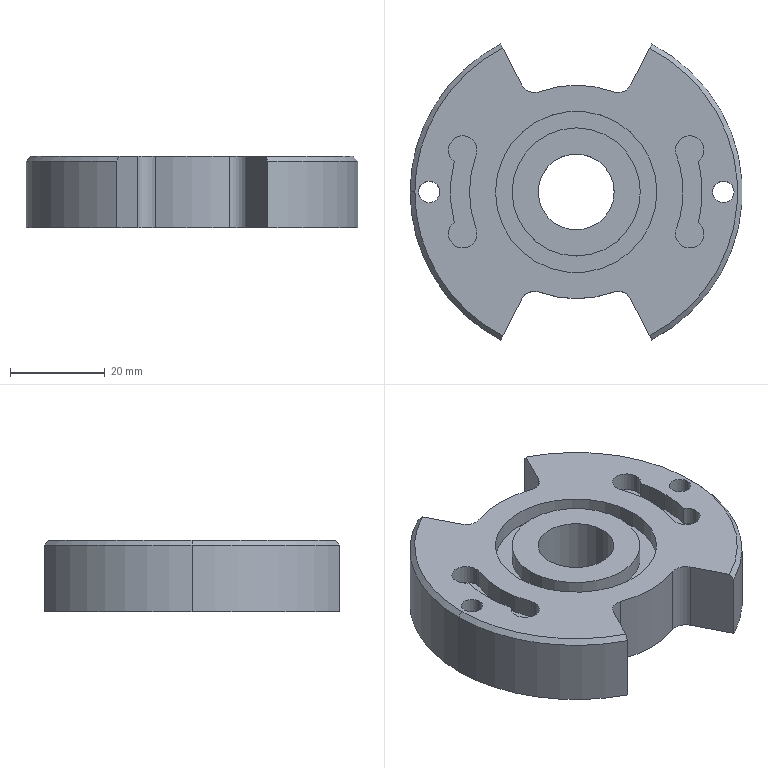Part | SolidWorks | features ICE 5, MirrorPattern 2, Chamfer 1, Extrusion 1, Fillet 1 | 1 solid | 50 faces | box 70 x 62.37 x 15 mm | volume 42070 mm3 | cylinder 37 | plane 10 | cone 3 | commonest cylinder face diameters 6 x16 45 x5 4.5 x4 53 x3 70 x3 16 x2
STEP:
#1=CARTESIAN_POINT('',(-34.,0.,15.));
#2=VERTEX_POINT('',#1);
#3=CARTESIAN_POINT('',(-15.436,-30.294,15.));
#4=VERTEX_POINT('',#3);
#5=CARTESIAN_POINT('',(0.,0.,15.));
#6=DIRECTION('',(0.,0.,1.));
#7=DIRECTION('',(1.,0.,0.));
#8=AXIS2_PLACEMENT_3D('',#5,#6,#7);
#9=CIRCLE('',#8,34.);
#10=EDGE_CURVE('',#2,#4,#9,.T.);
#11=ORIENTED_EDGE('',*,*,#10,.F.);
#12=CARTESIAN_POINT('',(-35.,0.,14.));
#13=VERTEX_POINT('',#12);
#14=CARTESIAN_POINT('',(-34.,0.,15.));
#15=DIRECTION('',(-0.7071,0.,-0.7071));
#16=VECTOR('',#15,1000.);
#17=LINE('',#14,#16);
#18=EDGE_CURVE('',#2,#13,#17,.T.);
#19=ORIENTED_EDGE('',*,*,#18,.T.);
#20=CARTESIAN_POINT('',(-15.89,-31.185,14.));
#21=VERTEX_POINT('',#20);
#22=CARTESIAN_POINT('',(0.,0.,14.));
#23=DIRECTION('',(0.,0.,-1.));
#24=DIRECTION('',(1.,0.,0.));
#25=AXIS2_PLACEMENT_3D('',#22,#23,#24);
#26=CIRCLE('',#25,35.);
#27=EDGE_CURVE('',#21,#13,#26,.T.);
#28=ORIENTED_EDGE('',*,*,#27,.F.);
#29=CARTESIAN_POINT('',(0.,0.,49.));
#30=DIRECTION('',(-0.321,-0.63,-0.7071));
#31=VECTOR('',#30,1000.);
#32=LINE('',#29,#31);
#33=EDGE_CURVE('',#4,#21,#32,.T.);
#34=ORIENTED_EDGE('',*,*,#33,.F.);
#35=EDGE_LOOP('',(#11,#19,#28,#34));
#36=FACE_OUTER_BOUND('',#35,.T.);
#37=CARTESIAN_POINT('',(0.,0.,15.));
#38=DIRECTION('',(0.,0.,-1.));
#39=DIRECTION('',(-1.,0.,0.));
#40=AXIS2_PLACEMENT_3D('',#37,#38,#39);
#41=CONICAL_SURFACE('',#40,34.,0.7854);
#42=ADVANCED_FACE('',(#36),#41,.T.);
#43=CARTESIAN_POINT('',(28.75,0.,0.));
#44=VERTEX_POINT('',#43);
#45=CARTESIAN_POINT('',(33.25,0.,0.));
#46=VERTEX_POINT('',#45);
#47=CARTESIAN_POINT('',(31.,0.,0.));
#48=DIRECTION('',(0.,0.,1.));
#49=DIRECTION('',(1.,0.,0.));
#50=AXIS2_PLACEMENT_3D('',#47,#48,#49);
#51=CIRCLE('',#50,2.25);
#52=EDGE_CURVE('',#44,#46,#51,.T.);
#53=ORIENTED_EDGE('',*,*,#52,.F.);
#54=CARTESIAN_POINT('',(28.75,0.,15.));
#55=VERTEX_POINT('',#54);
#56=CARTESIAN_POINT('',(28.75,0.,0.));
#57=DIRECTION('',(0.,0.,1.));
#58=VECTOR('',#57,1000.);
#59=LINE('',#56,#58);
#60=EDGE_CURVE('',#44,#55,#59,.T.);
#61=ORIENTED_EDGE('',*,*,#60,.T.);
#62=CARTESIAN_POINT('',(33.25,0.,15.));
#63=VERTEX_POINT('',#62);
#64=CARTESIAN_POINT('',(31.,0.,15.));
#65=DIRECTION('',(0.,0.,1.));
#66=DIRECTION('',(1.,0.,0.));
#67=AXIS2_PLACEMENT_3D('',#64,#65,#66);
#68=CIRCLE('',#67,2.25);
#69=EDGE_CURVE('',#55,#63,#68,.T.);
#70=ORIENTED_EDGE('',*,*,#69,.T.);
#71=CARTESIAN_POINT('',(33.25,0.,0.));
#72=DIRECTION('',(0.,0.,1.));
#73=VECTOR('',#72,1000.);
#74=LINE('',#71,#73);
#75=EDGE_CURVE('',#46,#63,#74,.T.);
#76=ORIENTED_EDGE('',*,*,#75,.F.);
#77=EDGE_LOOP('',(#53,#61,#70,#76));
#78=FACE_OUTER_BOUND('',#77,.T.);
#79=CARTESIAN_POINT('',(31.,0.,0.));
#80=DIRECTION('',(0.,0.,1.));
#81=DIRECTION('',(1.,0.,0.));
#82=AXIS2_PLACEMENT_3D('',#79,#80,#81);
#83=CYLINDRICAL_SURFACE('',#82,2.25);
#84=ADVANCED_FACE('',(#78),#83,.F.);
#85=CARTESIAN_POINT('',(-33.25,0.,0.));
#86=VERTEX_POINT('',#85);
#87=CARTESIAN_POINT('',(-28.75,0.,0.));
#88=VERTEX_POINT('',#87);
#89=CARTESIAN_POINT('',(-31.,0.,0.));
#90=DIRECTION('',(0.,0.,1.));
#91=DIRECTION('',(1.,0.,0.));
#92=AXIS2_PLACEMENT_3D('',#89,#90,#91);
#93=CIRCLE('',#92,2.25);
#94=EDGE_CURVE('',#86,#88,#93,.T.);
#95=ORIENTED_EDGE('',*,*,#94,.F.);
#96=CARTESIAN_POINT('',(-33.25,0.,15.));
#97=VERTEX_POINT('',#96);
#98=CARTESIAN_POINT('',(-33.25,0.,0.));
#99=DIRECTION('',(0.,0.,1.));
#100=VECTOR('',#99,1000.);
#101=LINE('',#98,#100);
#102=EDGE_CURVE('',#86,#97,#101,.T.);
#103=ORIENTED_EDGE('',*,*,#102,.T.);
#104=CARTESIAN_POINT('',(-28.75,0.,15.));
#105=VERTEX_POINT('',#104);
#106=CARTESIAN_POINT('',(-31.,0.,15.));
#107=DIRECTION('',(0.,0.,1.));
#108=DIRECTION('',(1.,0.,0.));
#109=AXIS2_PLACEMENT_3D('',#106,#107,#108);
#110=CIRCLE('',#109,2.25);
#111=EDGE_CURVE('',#97,#105,#110,.T.);
#112=ORIENTED_EDGE('',*,*,#111,.T.);
#113=CARTESIAN_POINT('',(-28.75,0.,0.));
#114=DIRECTION('',(0.,0.,1.));
#115=VECTOR('',#114,1000.);
#116=LINE('',#113,#115);
#117=EDGE_CURVE('',#88,#105,#116,.T.);
#118=ORIENTED_EDGE('',*,*,#117,.F.);
#119=EDGE_LOOP('',(#95,#103,#112,#118));
#120=FACE_OUTER_BOUND('',#119,.T.);
#121=CARTESIAN_POINT('',(-31.,0.,0.));
#122=DIRECTION('',(0.,0.,1.));
#123=DIRECTION('',(1.,0.,0.));
#124=AXIS2_PLACEMENT_3D('',#121,#122,#123);
#125=CYLINDRICAL_SURFACE('',#124,2.25);
#126=ADVANCED_FACE('',(#120),#125,.F.);
#127=CARTESIAN_POINT('',(-8.,0.,0.));
#128=VERTEX_POINT('',#127);
#129=CARTESIAN_POINT('',(8.,0.,0.));
#130=VERTEX_POINT('',#129);
#131=CARTESIAN_POINT('',(0.,0.,0.));
#132=DIRECTION('',(0.,0.,1.));
#133=DIRECTION('',(1.,0.,0.));
#134=AXIS2_PLACEMENT_3D('',#131,#132,#133);
#135=CIRCLE('',#134,8.);
#136=EDGE_CURVE('',#128,#130,#135,.T.);
#137=ORIENTED_EDGE('',*,*,#136,.F.);
#138=CARTESIAN_POINT('',(-8.,0.,15.));
#139=VERTEX_POINT('',#138);
#140=CARTESIAN_POINT('',(-8.,0.,0.));
#141=DIRECTION('',(0.,0.,1.));
#142=VECTOR('',#141,1000.);
#143=LINE('',#140,#142);
#144=EDGE_CURVE('',#128,#139,#143,.T.);
#145=ORIENTED_EDGE('',*,*,#144,.T.);
#146=CARTESIAN_POINT('',(8.,0.,15.));
#147=VERTEX_POINT('',#146);
#148=CARTESIAN_POINT('',(0.,0.,15.));
#149=DIRECTION('',(0.,0.,1.));
#150=DIRECTION('',(1.,0.,0.));
#151=AXIS2_PLACEMENT_3D('',#148,#149,#150);
#152=CIRCLE('',#151,8.);
#153=EDGE_CURVE('',#139,#147,#152,.T.);
#154=ORIENTED_EDGE('',*,*,#153,.T.);
#155=CARTESIAN_POINT('',(8.,0.,0.));
#156=DIRECTION('',(0.,0.,1.));
#157=VECTOR('',#156,1000.);
#158=LINE('',#155,#157);
#159=EDGE_CURVE('',#130,#147,#158,.T.);
#160=ORIENTED_EDGE('',*,*,#159,.F.);
#161=EDGE_LOOP('',(#137,#145,#154,#160));
#162=FACE_OUTER_BOUND('',#161,.T.);
#163=CARTESIAN_POINT('',(0.,0.,0.));
#164=DIRECTION('',(0.,0.,1.));
#165=DIRECTION('',(1.,0.,0.));
#166=AXIS2_PLACEMENT_3D('',#163,#164,#165);
#167=CYLINDRICAL_SURFACE('',#166,8.);
#168=ADVANCED_FACE('',(#162),#167,.F.);
#169=CARTESIAN_POINT('',(-25.712,6.414,11.));
#170=VERTEX_POINT('',#169);
#171=CARTESIAN_POINT('',(-26.925,8.823,11.));
#172=VERTEX_POINT('',#171);
#173=CARTESIAN_POINT('',(-23.925,8.823,11.));
#174=DIRECTION('',(0.,0.,-1.));
#175=DIRECTION('',(-1.,0.,0.));
#176=AXIS2_PLACEMENT_3D('',#173,#174,#175);
#177=CIRCLE('',#176,3.);
#178=EDGE_CURVE('',#170,#172,#177,.T.);
#179=ORIENTED_EDGE('',*,*,#178,.T.);
#180=CARTESIAN_POINT('',(-26.925,8.823,15.));
#181=VERTEX_POINT('',#180);
#182=CARTESIAN_POINT('',(-26.925,8.823,11.));
#183=DIRECTION('',(0.,0.,1.));
#184=VECTOR('',#183,1000.);
#185=LINE('',#182,#184);
#186=EDGE_CURVE('',#172,#181,#185,.T.);
#187=ORIENTED_EDGE('',*,*,#186,.T.);
#188=CARTESIAN_POINT('',(-25.712,6.414,15.));
#189=VERTEX_POINT('',#188);
#190=CARTESIAN_POINT('',(-23.925,8.823,15.));
#191=DIRECTION('',(0.,0.,-1.));
#192=DIRECTION('',(-1.,0.,0.));
#193=AXIS2_PLACEMENT_3D('',#190,#191,#192);
#194=CIRCLE('',#193,3.);
#195=EDGE_CURVE('',#189,#181,#194,.T.);
#196=ORIENTED_EDGE('',*,*,#195,.F.);
#197=CARTESIAN_POINT('',(-25.712,6.414,11.));
#198=DIRECTION('',(0.,0.,1.));
#199=VECTOR('',#198,1000.);
#200=LINE('',#197,#199);
#201=EDGE_CURVE('',#170,#189,#200,.T.);
#202=ORIENTED_EDGE('',*,*,#201,.F.);
#203=EDGE_LOOP('',(#179,#187,#196,#202));
#204=FACE_OUTER_BOUND('',#203,.T.);
#205=CARTESIAN_POINT('',(-23.925,8.823,11.));
#206=DIRECTION('',(0.,0.,1.));
#207=DIRECTION('',(1.,0.,0.));
#208=AXIS2_PLACEMENT_3D('',#205,#206,#207);
#209=CYLINDRICAL_SURFACE('',#208,3.);
#210=ADVANCED_FACE('',(#204),#209,.F.);
#211=ORIENTED_EDGE('',*,*,#186,.F.);
#212=CARTESIAN_POINT('',(-20.925,8.823,11.));
#213=VERTEX_POINT('',#212);
#214=CARTESIAN_POINT('',(-23.925,8.823,11.));
#215=DIRECTION('',(0.,0.,-1.));
#216=DIRECTION('',(-1.,0.,0.));
#217=AXIS2_PLACEMENT_3D('',#214,#215,#216);
#218=CIRCLE('',#217,3.);
#219=EDGE_CURVE('',#172,#213,#218,.T.);
#220=ORIENTED_EDGE('',*,*,#219,.T.);
#221=CARTESIAN_POINT('',(-20.925,8.823,15.));
#222=VERTEX_POINT('',#221);
#223=CARTESIAN_POINT('',(-20.925,8.823,11.));
#224=DIRECTION('',(0.,0.,1.));
#225=VECTOR('',#224,1000.);
#226=LINE('',#223,#225);
#227=EDGE_CURVE('',#213,#222,#226,.T.);
#228=ORIENTED_EDGE('',*,*,#227,.T.);
#229=CARTESIAN_POINT('',(-23.925,8.823,15.));
#230=DIRECTION('',(0.,0.,-1.));
#231=DIRECTION('',(-1.,0.,0.));
#232=AXIS2_PLACEMENT_3D('',#229,#230,#231);
#233=CIRCLE('',#232,3.);
#234=EDGE_CURVE('',#181,#222,#233,.T.);
#235=ORIENTED_EDGE('',*,*,#234,.F.);
#236=EDGE_LOOP('',(#211,#220,#228,#235));
#237=FACE_OUTER_BOUND('',#236,.T.);
#238=CARTESIAN_POINT('',(-23.925,8.823,11.));
#239=DIRECTION('',(0.,0.,1.));
#240=DIRECTION('',(1.,0.,0.));
#241=AXIS2_PLACEMENT_3D('',#238,#239,#240);
#242=CYLINDRICAL_SURFACE('',#241,3.);
#243=ADVANCED_FACE('',(#237),#242,.F.);
#244=CARTESIAN_POINT('',(-20.925,-8.823,11.));
#245=VERTEX_POINT('',#244);
#246=CARTESIAN_POINT('',(-26.925,-8.823,11.));
#247=VERTEX_POINT('',#246);
#248=CARTESIAN_POINT('',(-23.925,-8.823,11.));
#249=DIRECTION('',(0.,0.,-1.));
#250=DIRECTION('',(-1.,0.,0.));
#251=AXIS2_PLACEMENT_3D('',#248,#249,#250);
#252=CIRCLE('',#251,3.);
#253=EDGE_CURVE('',#245,#247,#252,.T.);
#254=ORIENTED_EDGE('',*,*,#253,.T.);
#255=CARTESIAN_POINT('',(-26.925,-8.823,15.));
#256=VERTEX_POINT('',#255);
#257=CARTESIAN_POINT('',(-26.925,-8.823,11.));
#258=DIRECTION('',(0.,0.,1.));
#259=VECTOR('',#258,1000.);
#260=LINE('',#257,#259);
#261=EDGE_CURVE('',#247,#256,#260,.T.);
#262=ORIENTED_EDGE('',*,*,#261,.T.);
#263=CARTESIAN_POINT('',(-20.925,-8.823,15.));
#264=VERTEX_POINT('',#263);
#265=CARTESIAN_POINT('',(-23.925,-8.823,15.));
#266=DIRECTION('',(0.,0.,-1.));
#267=DIRECTION('',(-1.,0.,0.));
#268=AXIS2_PLACEMENT_3D('',#265,#266,#267);
#269=CIRCLE('',#268,3.);
#270=EDGE_CURVE('',#264,#256,#269,.T.);
#271=ORIENTED_EDGE('',*,*,#270,.F.);
#272=CARTESIAN_POINT('',(-20.925,-8.823,11.));
#273=DIRECTION('',(0.,0.,1.));
#274=VECTOR('',#273,1000.);
#275=LINE('',#272,#274);
#276=EDGE_CURVE('',#245,#264,#275,.T.);
#277=ORIENTED_EDGE('',*,*,#276,.F.);
#278=EDGE_LOOP('',(#254,#262,#271,#277));
#279=FACE_OUTER_BOUND('',#278,.T.);
#280=CARTESIAN_POINT('',(-23.925,-8.823,11.));
#281=DIRECTION('',(0.,0.,1.));
#282=DIRECTION('',(1.,0.,0.));
#283=AXIS2_PLACEMENT_3D('',#280,#281,#282);
#284=CYLINDRICAL_SURFACE('',#283,3.);
#285=ADVANCED_FACE('',(#279),#284,.F.);
#286=CARTESIAN_POINT('',(-21.11,-7.785,11.));
#287=VERTEX_POINT('',#286);
#288=CARTESIAN_POINT('',(-23.925,-8.823,11.));
#289=DIRECTION('',(0.,0.,-1.));
#290=DIRECTION('',(-1.,0.,0.));
#291=AXIS2_PLACEMENT_3D('',#288,#289,#290);
#292=CIRCLE('',#291,3.);
#293=EDGE_CURVE('',#287,#245,#292,.T.);
#294=ORIENTED_EDGE('',*,*,#293,.T.);
#295=ORIENTED_EDGE('',*,*,#276,.T.);
#296=CARTESIAN_POINT('',(-21.11,-7.785,15.));
#297=VERTEX_POINT('',#296);
#298=CARTESIAN_POINT('',(-23.925,-8.823,15.));
#299=DIRECTION('',(0.,0.,-1.));
#300=DIRECTION('',(-1.,0.,0.));
#301=AXIS2_PLACEMENT_3D('',#298,#299,#300);
#302=CIRCLE('',#301,3.);
#303=EDGE_CURVE('',#297,#264,#302,.T.);
#304=ORIENTED_EDGE('',*,*,#303,.F.);
#305=CARTESIAN_POINT('',(-21.11,-7.785,11.));
#306=DIRECTION('',(0.,0.,1.));
#307=VECTOR('',#306,1000.);
#308=LINE('',#305,#307);
#309=EDGE_CURVE('',#287,#297,#308,.T.);
#310=ORIENTED_EDGE('',*,*,#309,.F.);
#311=EDGE_LOOP('',(#294,#295,#304,#310));
#312=FACE_OUTER_BOUND('',#311,.T.);
#313=CARTESIAN_POINT('',(-23.925,-8.823,11.));
#314=DIRECTION('',(0.,0.,1.));
#315=DIRECTION('',(1.,0.,0.));
#316=AXIS2_PLACEMENT_3D('',#313,#314,#315);
#317=CYLINDRICAL_SURFACE('',#316,3.);
#318=ADVANCED_FACE('',(#312),#317,.F.);
#319=CARTESIAN_POINT('',(26.5,0.,11.));
#320=VERTEX_POINT('',#319);
#321=CARTESIAN_POINT('',(25.712,6.414,11.));
#322=VERTEX_POINT('',#321);
#323=CARTESIAN_POINT('',(0.,0.,11.));
#324=DIRECTION('',(0.,0.,1.));
#325=DIRECTION('',(-1.,0.,0.));
#326=AXIS2_PLACEMENT_3D('',#323,#324,#325);
#327=CIRCLE('',#326,26.5);
#328=EDGE_CURVE('',#320,#322,#327,.T.);
#329=ORIENTED_EDGE('',*,*,#328,.F.);
#330=CARTESIAN_POINT('',(26.5,0.,15.));
#331=VERTEX_POINT('',#330);
#332=CARTESIAN_POINT('',(26.5,0.,11.));
#333=DIRECTION('',(0.,0.,1.));
#334=VECTOR('',#333,1000.);
#335=LINE('',#332,#334);
#336=EDGE_CURVE('',#320,#331,#335,.T.);
#337=ORIENTED_EDGE('',*,*,#336,.T.);
#338=CARTESIAN_POINT('',(25.712,6.414,15.));
#339=VERTEX_POINT('',#338);
#340=CARTESIAN_POINT('',(0.,0.,15.));
#341=DIRECTION('',(0.,0.,1.));
#342=DIRECTION('',(-1.,0.,0.));
#343=AXIS2_PLACEMENT_3D('',#340,#341,#342);
#344=CIRCLE('',#343,26.5);
#345=EDGE_CURVE('',#331,#339,#344,.T.);
#346=ORIENTED_EDGE('',*,*,#345,.T.);
#347=CARTESIAN_POINT('',(25.712,6.414,11.));
#348=DIRECTION('',(0.,0.,1.));
#349=VECTOR('',#348,1000.);
#350=LINE('',#347,#349);
#351=EDGE_CURVE('',#322,#339,#350,.T.);
#352=ORIENTED_EDGE('',*,*,#351,.F.);
#353=EDGE_LOOP('',(#329,#337,#346,#352));
#354=FACE_OUTER_BOUND('',#353,.T.);
#355=CARTESIAN_POINT('',(0.,0.,11.));
#356=DIRECTION('',(0.,0.,1.));
#357=DIRECTION('',(1.,0.,0.));
#358=AXIS2_PLACEMENT_3D('',#355,#356,#357);
#359=CYLINDRICAL_SURFACE('',#358,26.5);
#360=ADVANCED_FACE('',(#354),#359,.F.);
#361=CARTESIAN_POINT('',(20.925,8.823,11.));
#362=VERTEX_POINT('',#361);
#363=CARTESIAN_POINT('',(21.11,7.785,11.));
#364=VERTEX_POINT('',#363);
#365=CARTESIAN_POINT('',(23.925,8.823,11.));
#366=DIRECTION('',(0.,0.,1.));
#367=DIRECTION('',(1.,0.,0.));
#368=AXIS2_PLACEMENT_3D('',#365,#366,#367);
#369=CIRCLE('',#368,3.);
#370=EDGE_CURVE('',#362,#364,#369,.T.);
#371=ORIENTED_EDGE('',*,*,#370,.F.);
#372=CARTESIAN_POINT('',(20.925,8.823,15.));
#373=VERTEX_POINT('',#372);
#374=CARTESIAN_POINT('',(20.925,8.823,11.));
#375=DIRECTION('',(0.,0.,1.));
#376=VECTOR('',#375,1000.);
#377=LINE('',#374,#376);
#378=EDGE_CURVE('',#362,#373,#377,.T.);
#379=ORIENTED_EDGE('',*,*,#378,.T.);
#380=CARTESIAN_POINT('',(21.11,7.785,15.));
#381=VERTEX_POINT('',#380);
#382=CARTESIAN_POINT('',(23.925,8.823,15.));
#383=DIRECTION('',(0.,0.,1.));
#384=DIRECTION('',(1.,0.,0.));
#385=AXIS2_PLACEMENT_3D('',#382,#383,#384);
#386=CIRCLE('',#385,3.);
#387=EDGE_CURVE('',#373,#381,#386,.T.);
#388=ORIENTED_EDGE('',*,*,#387,.T.);
#389=CARTESIAN_POINT('',(21.11,7.785,11.));
#390=DIRECTION('',(0.,0.,1.));
#391=VECTOR('',#390,1000.);
#392=LINE('',#389,#391);
#393=EDGE_CURVE('',#364,#381,#392,.T.);
#394=ORIENTED_EDGE('',*,*,#393,.F.);
#395=EDGE_LOOP('',(#371,#379,#388,#394));
#396=FACE_OUTER_BOUND('',#395,.T.);
#397=CARTESIAN_POINT('',(23.925,8.823,11.));
#398=DIRECTION('',(0.,0.,1.));
#399=DIRECTION('',(1.,0.,0.));
#400=AXIS2_PLACEMENT_3D('',#397,#398,#399);
#401=CYLINDRICAL_SURFACE('',#400,3.);
#402=ADVANCED_FACE('',(#396),#401,.F.);
#403=ORIENTED_EDGE('',*,*,#378,.F.);
#404=CARTESIAN_POINT('',(26.925,8.823,11.));
#405=VERTEX_POINT('',#404);
#406=CARTESIAN_POINT('',(23.925,8.823,11.));
#407=DIRECTION('',(0.,0.,1.));
#408=DIRECTION('',(1.,0.,0.));
#409=AXIS2_PLACEMENT_3D('',#406,#407,#408);
#410=CIRCLE('',#409,3.);
#411=EDGE_CURVE('',#405,#362,#410,.T.);
#412=ORIENTED_EDGE('',*,*,#411,.F.);
#413=CARTESIAN_POINT('',(26.925,8.823,15.));
#414=VERTEX_POINT('',#413);
#415=CARTESIAN_POINT('',(26.925,8.823,11.));
#416=DIRECTION('',(0.,0.,1.));
#417=VECTOR('',#416,1000.);
#418=LINE('',#415,#417);
#419=EDGE_CURVE('',#405,#414,#418,.T.);
#420=ORIENTED_EDGE('',*,*,#419,.T.);
#421=CARTESIAN_POINT('',(23.925,8.823,15.));
#422=DIRECTION('',(0.,0.,1.));
#423=DIRECTION('',(1.,0.,0.));
#424=AXIS2_PLACEMENT_3D('',#421,#422,#423);
#425=CIRCLE('',#424,3.);
#426=EDGE_CURVE('',#414,#373,#425,.T.);
#427=ORIENTED_EDGE('',*,*,#426,.T.);
#428=EDGE_LOOP('',(#403,#412,#420,#427));
#429=FACE_OUTER_BOUND('',#428,.T.);
#430=CARTESIAN_POINT('',(23.925,8.823,11.));
#431=DIRECTION('',(0.,0.,1.));
#432=DIRECTION('',(1.,0.,0.));
#433=AXIS2_PLACEMENT_3D('',#430,#431,#432);
#434=CYLINDRICAL_SURFACE('',#433,3.);
#435=ADVANCED_FACE('',(#429),#434,.F.);
#436=CARTESIAN_POINT('',(22.5,0.,11.));
#437=VERTEX_POINT('',#436);
#438=CARTESIAN_POINT('',(21.11,-7.785,11.));
#439=VERTEX_POINT('',#438);
#440=CARTESIAN_POINT('',(0.,0.,11.));
#441=DIRECTION('',(0.,0.,-1.));
#442=DIRECTION('',(-1.,0.,0.));
#443=AXIS2_PLACEMENT_3D('',#440,#441,#442);
#444=CIRCLE('',#443,22.5);
#445=EDGE_CURVE('',#437,#439,#444,.T.);
#446=ORIENTED_EDGE('',*,*,#445,.F.);
#447=CARTESIAN_POINT('',(22.5,0.,15.));
#448=VERTEX_POINT('',#447);
#449=CARTESIAN_POINT('',(22.5,0.,11.));
#450=DIRECTION('',(0.,0.,1.));
#451=VECTOR('',#450,1000.);
#452=LINE('',#449,#451);
#453=EDGE_CURVE('',#437,#448,#452,.T.);
#454=ORIENTED_EDGE('',*,*,#453,.T.);
#455=CARTESIAN_POINT('',(21.11,-7.785,15.));
#456=VERTEX_POINT('',#455);
#457=CARTESIAN_POINT('',(0.,0.,15.));
#458=DIRECTION('',(0.,0.,-1.));
#459=DIRECTION('',(-1.,0.,0.));
#460=AXIS2_PLACEMENT_3D('',#457,#458,#459);
#461=CIRCLE('',#460,22.5);
#462=EDGE_CURVE('',#448,#456,#461,.T.);
#463=ORIENTED_EDGE('',*,*,#462,.T.);
#464=CARTESIAN_POINT('',(21.11,-7.785,11.));
#465=DIRECTION('',(0.,0.,1.));
#466=VECTOR('',#465,1000.);
#467=LINE('',#464,#466);
#468=EDGE_CURVE('',#439,#456,#467,.T.);
#469=ORIENTED_EDGE('',*,*,#468,.F.);
#470=EDGE_LOOP('',(#446,#454,#463,#469));
#471=FACE_OUTER_BOUND('',#470,.T.);
#472=CARTESIAN_POINT('',(0.,0.,11.));
#473=DIRECTION('',(0.,0.,1.));
#474=DIRECTION('',(1.,0.,0.));
#475=AXIS2_PLACEMENT_3D('',#472,#473,#474);
#476=CYLINDRICAL_SURFACE('',#475,22.5);
#477=ADVANCED_FACE('',(#471),#476,.T.);
#478=CARTESIAN_POINT('',(20.925,-8.823,11.));
#479=VERTEX_POINT('',#478);
#480=CARTESIAN_POINT('',(26.925,-8.823,11.));
#481=VERTEX_POINT('',#480);
#482=CARTESIAN_POINT('',(23.925,-8.823,11.));
#483=DIRECTION('',(0.,0.,1.));
#484=DIRECTION('',(1.,0.,0.));
#485=AXIS2_PLACEMENT_3D('',#482,#483,#484);
#486=CIRCLE('',#485,3.);
#487=EDGE_CURVE('',#479,#481,#486,.T.);
#488=ORIENTED_EDGE('',*,*,#487,.F.);
#489=CARTESIAN_POINT('',(20.925,-8.823,15.));
#490=VERTEX_POINT('',#489);
#491=CARTESIAN_POINT('',(20.925,-8.823,11.));
#492=DIRECTION('',(0.,0.,1.));
#493=VECTOR('',#492,1000.);
#494=LINE('',#491,#493);
#495=EDGE_CURVE('',#479,#490,#494,.T.);
#496=ORIENTED_EDGE('',*,*,#495,.T.);
#497=CARTESIAN_POINT('',(26.925,-8.823,15.));
#498=VERTEX_POINT('',#497);
#499=CARTESIAN_POINT('',(23.925,-8.823,15.));
#500=DIRECTION('',(0.,0.,1.));
#501=DIRECTION('',(1.,0.,0.));
#502=AXIS2_PLACEMENT_3D('',#499,#500,#501);
#503=CIRCLE('',#502,3.);
#504=EDGE_CURVE('',#490,#498,#503,.T.);
#505=ORIENTED_EDGE('',*,*,#504,.T.);
#506=CARTESIAN_POINT('',(26.925,-8.823,11.));
#507=DIRECTION('',(0.,0.,1.));
#508=VECTOR('',#507,1000.);
#509=LINE('',#506,#508);
#510=EDGE_CURVE('',#481,#498,#509,.T.);
#511=ORIENTED_EDGE('',*,*,#510,.F.);
#512=EDGE_LOOP('',(#488,#496,#505,#511));
#513=FACE_OUTER_BOUND('',#512,.T.);
#514=CARTESIAN_POINT('',(23.925,-8.823,11.));
#515=DIRECTION('',(0.,0.,1.));
#516=DIRECTION('',(1.,0.,0.));
#517=AXIS2_PLACEMENT_3D('',#514,#515,#516);
#518=CYLINDRICAL_SURFACE('',#517,3.);
#519=ADVANCED_FACE('',(#513),#518,.F.);
#520=CARTESIAN_POINT('',(25.712,-6.414,11.));
#521=VERTEX_POINT('',#520);
#522=CARTESIAN_POINT('',(23.925,-8.823,11.));
#523=DIRECTION('',(0.,0.,1.));
#524=DIRECTION('',(1.,0.,0.));
#525=AXIS2_PLACEMENT_3D('',#522,#523,#524);
#526=CIRCLE('',#525,3.);
#527=EDGE_CURVE('',#481,#521,#526,.T.);
#528=ORIENTED_EDGE('',*,*,#527,.F.);
#529=ORIENTED_EDGE('',*,*,#510,.T.);
#530=CARTESIAN_POINT('',(25.712,-6.414,15.));
#531=VERTEX_POINT('',#530);
#532=CARTESIAN_POINT('',(23.925,-8.823,15.));
#533=DIRECTION('',(0.,0.,1.));
#534=DIRECTION('',(1.,0.,0.));
#535=AXIS2_PLACEMENT_3D('',#532,#533,#534);
#536=CIRCLE('',#535,3.);
#537=EDGE_CURVE('',#498,#531,#536,.T.);
#538=ORIENTED_EDGE('',*,*,#537,.T.);
#539=CARTESIAN_POINT('',(25.712,-6.414,11.));
#540=DIRECTION('',(0.,0.,1.));
#541=VECTOR('',#540,1000.);
#542=LINE('',#539,#541);
#543=EDGE_CURVE('',#521,#531,#542,.T.);
#544=ORIENTED_EDGE('',*,*,#543,.F.);
#545=EDGE_LOOP('',(#528,#529,#538,#544));
#546=FACE_OUTER_BOUND('',#545,.T.);
#547=CARTESIAN_POINT('',(23.925,-8.823,11.));
#548=DIRECTION('',(0.,0.,1.));
#549=DIRECTION('',(1.,0.,0.));
#550=AXIS2_PLACEMENT_3D('',#547,#548,#549);
#551=CYLINDRICAL_SURFACE('',#550,3.);
#552=ADVANCED_FACE('',(#546),#551,.F.);
#553=CARTESIAN_POINT('',(13.5,0.,11.5));
#554=VERTEX_POINT('',#553);
#555=CARTESIAN_POINT('',(-13.5,0.,11.5));
#556=VERTEX_POINT('',#555);
#557=CARTESIAN_POINT('',(0.,0.,11.5));
#558=DIRECTION('',(0.,0.,1.));
#559=DIRECTION('',(1.,0.,0.));
#560=AXIS2_PLACEMENT_3D('',#557,#558,#559);
#561=CIRCLE('',#560,13.5);
#562=EDGE_CURVE('',#554,#556,#561,.T.);
#563=ORIENTED_EDGE('',*,*,#562,.T.);
#564=CARTESIAN_POINT('',(-13.5,0.,15.));
#565=VERTEX_POINT('',#564);
#566=CARTESIAN_POINT('',(-13.5,0.,11.5));
#567=DIRECTION('',(0.,0.,1.));
#568=VECTOR('',#567,1000.);
#569=LINE('',#566,#568);
#570=EDGE_CURVE('',#556,#565,#569,.T.);
#571=ORIENTED_EDGE('',*,*,#570,.T.);
#572=CARTESIAN_POINT('',(13.5,0.,15.));
#573=VERTEX_POINT('',#572);
#574=CARTESIAN_POINT('',(0.,0.,15.));
#575=DIRECTION('',(0.,0.,1.));
#576=DIRECTION('',(1.,0.,0.));
#577=AXIS2_PLACEMENT_3D('',#574,#575,#576);
#578=CIRCLE('',#577,13.5);
#579=EDGE_CURVE('',#573,#565,#578,.T.);
#580=ORIENTED_EDGE('',*,*,#579,.F.);
#581=CARTESIAN_POINT('',(13.5,0.,11.5));
#582=DIRECTION('',(0.,0.,1.));
#583=VECTOR('',#582,1000.);
#584=LINE('',#581,#583);
#585=EDGE_CURVE('',#554,#573,#584,.T.);
#586=ORIENTED_EDGE('',*,*,#585,.F.);
#587=EDGE_LOOP('',(#563,#571,#580,#586));
#588=FACE_OUTER_BOUND('',#587,.T.);
#589=CARTESIAN_POINT('',(0.,0.,11.5));
#590=DIRECTION('',(0.,0.,1.));
#591=DIRECTION('',(1.,0.,0.));
#592=AXIS2_PLACEMENT_3D('',#589,#590,#591);
#593=CYLINDRICAL_SURFACE('',#592,13.5);
#594=ADVANCED_FACE('',(#588),#593,.T.);
#595=CARTESIAN_POINT('',(-17.,0.,11.5));
#596=VERTEX_POINT('',#595);
#597=CARTESIAN_POINT('',(17.,0.,11.5));
#598=VERTEX_POINT('',#597);
#599=CARTESIAN_POINT('',(0.,0.,11.5));
#600=DIRECTION('',(0.,0.,1.));
#601=DIRECTION('',(1.,0.,0.));
#602=AXIS2_PLACEMENT_3D('',#599,#600,#601);
#603=CIRCLE('',#602,17.);
#604=EDGE_CURVE('',#596,#598,#603,.T.);
#605=ORIENTED_EDGE('',*,*,#604,.F.);
#606=CARTESIAN_POINT('',(-17.,0.,15.));
#607=VERTEX_POINT('',#606);
#608=CARTESIAN_POINT('',(-17.,0.,11.5));
#609=DIRECTION('',(0.,0.,1.));
#610=VECTOR('',#609,1000.);
#611=LINE('',#608,#610);
#612=EDGE_CURVE('',#596,#607,#611,.T.);
#613=ORIENTED_EDGE('',*,*,#612,.T.);
#614=CARTESIAN_POINT('',(17.,0.,15.));
#615=VERTEX_POINT('',#614);
#616=CARTESIAN_POINT('',(0.,0.,15.));
#617=DIRECTION('',(0.,0.,1.));
#618=DIRECTION('',(1.,0.,0.));
#619=AXIS2_PLACEMENT_3D('',#616,#617,#618);
#620=CIRCLE('',#619,17.);
#621=EDGE_CURVE('',#607,#615,#620,.T.);
#622=ORIENTED_EDGE('',*,*,#621,.T.);
#623=CARTESIAN_POINT('',(17.,0.,11.5));
#624=DIRECTION('',(0.,0.,1.));
#625=VECTOR('',#624,1000.);
#626=LINE('',#623,#625);
#627=EDGE_CURVE('',#598,#615,#626,.T.);
#628=ORIENTED_EDGE('',*,*,#627,.F.);
#629=EDGE_LOOP('',(#605,#613,#622,#628));
#630=FACE_OUTER_BOUND('',#629,.T.);
#631=CARTESIAN_POINT('',(0.,0.,11.5));
#632=DIRECTION('',(0.,0.,1.));
#633=DIRECTION('',(1.,0.,0.));
#634=AXIS2_PLACEMENT_3D('',#631,#632,#633);
#635=CYLINDRICAL_SURFACE('',#634,17.);
#636=ADVANCED_FACE('',(#630),#635,.F.);
#637=ORIENTED_EDGE('',*,*,#27,.T.);
#638=CARTESIAN_POINT('',(-35.,0.,0.));
#639=VERTEX_POINT('',#638);
#640=CARTESIAN_POINT('',(-35.,0.,15.));
#641=DIRECTION('',(0.,0.,-1.));
#642=VECTOR('',#641,1000.);
#643=LINE('',#640,#642);
#644=EDGE_CURVE('',#13,#639,#643,.T.);
#645=ORIENTED_EDGE('',*,*,#644,.T.);
#646=CARTESIAN_POINT('',(-15.89,-31.185,0.));
#647=VERTEX_POINT('',#646);
#648=CARTESIAN_POINT('',(0.,0.,0.));
#649=DIRECTION('',(0.,0.,1.));
#650=DIRECTION('',(1.,0.,0.));
#651=AXIS2_PLACEMENT_3D('',#648,#649,#650);
#652=CIRCLE('',#651,35.);
#653=EDGE_CURVE('',#639,#647,#652,.T.);
#654=ORIENTED_EDGE('',*,*,#653,.T.);
#655=CARTESIAN_POINT('',(-15.89,-31.185,15.));
#656=DIRECTION('',(0.,0.,-1.));
#657=VECTOR('',#656,1000.);
#658=LINE('',#655,#657);
#659=EDGE_CURVE('',#21,#647,#658,.T.);
#660=ORIENTED_EDGE('',*,*,#659,.F.);
#661=EDGE_LOOP('',(#637,#645,#654,#660));
#662=FACE_OUTER_BOUND('',#661,.T.);
#663=CARTESIAN_POINT('',(0.,0.,15.));
#664=DIRECTION('',(0.,0.,-1.));
#665=DIRECTION('',(-1.,0.,0.));
#666=AXIS2_PLACEMENT_3D('',#663,#664,#665);
#667=CYLINDRICAL_SURFACE('',#666,35.);
#668=ADVANCED_FACE('',(#662),#667,.T.);
#669=CARTESIAN_POINT('',(31.,0.,15.));
#670=DIRECTION('',(0.,0.,1.));
#671=DIRECTION('',(1.,0.,0.));
#672=AXIS2_PLACEMENT_3D('',#669,#670,#671);
#673=CIRCLE('',#672,2.25);
#674=EDGE_CURVE('',#63,#55,#673,.T.);
#675=ORIENTED_EDGE('',*,*,#674,.F.);
#676=ORIENTED_EDGE('',*,*,#69,.F.);
#677=EDGE_LOOP('',(#675,#676));
#678=FACE_BOUND('',#677,.T.);
#679=CARTESIAN_POINT('',(-31.,0.,15.));
#680=DIRECTION('',(0.,0.,1.));
#681=DIRECTION('',(1.,0.,0.));
#682=AXIS2_PLACEMENT_3D('',#679,#680,#681);
#683=CIRCLE('',#682,2.25);
#684=EDGE_CURVE('',#105,#97,#683,.T.);
#685=ORIENTED_EDGE('',*,*,#684,.F.);
#686=ORIENTED_EDGE('',*,*,#111,.F.);
#687=EDGE_LOOP('',(#685,#686));
#688=FACE_BOUND('',#687,.T.);
#689=CARTESIAN_POINT('',(23.925,-8.823,15.));
#690=DIRECTION('',(0.,0.,1.));
#691=DIRECTION('',(1.,0.,0.));
#692=AXIS2_PLACEMENT_3D('',#689,#690,#691);
#693=CIRCLE('',#692,3.);
#694=EDGE_CURVE('',#456,#490,#693,.T.);
#695=ORIENTED_EDGE('',*,*,#694,.F.);
#696=ORIENTED_EDGE('',*,*,#462,.F.);
#697=CARTESIAN_POINT('',(0.,0.,15.));
#698=DIRECTION('',(0.,0.,-1.));
#699=DIRECTION('',(-1.,0.,0.));
#700=AXIS2_PLACEMENT_3D('',#697,#698,#699);
#701=CIRCLE('',#700,22.5);
#702=EDGE_CURVE('',#381,#448,#701,.T.);
#703=ORIENTED_EDGE('',*,*,#702,.F.);
#704=ORIENTED_EDGE('',*,*,#387,.F.);
#705=ORIENTED_EDGE('',*,*,#426,.F.);
#706=CARTESIAN_POINT('',(23.925,8.823,15.));
#707=DIRECTION('',(0.,0.,1.));
#708=DIRECTION('',(1.,0.,0.));
#709=AXIS2_PLACEMENT_3D('',#706,#707,#708);
#710=CIRCLE('',#709,3.);
#711=EDGE_CURVE('',#339,#414,#710,.T.);
#712=ORIENTED_EDGE('',*,*,#711,.F.);
#713=ORIENTED_EDGE('',*,*,#345,.F.);
#714=CARTESIAN_POINT('',(0.,0.,15.));
#715=DIRECTION('',(0.,0.,1.));
#716=DIRECTION('',(-1.,0.,0.));
#717=AXIS2_PLACEMENT_3D('',#714,#715,#716);
#718=CIRCLE('',#717,26.5);
#719=EDGE_CURVE('',#531,#331,#718,.T.);
#720=ORIENTED_EDGE('',*,*,#719,.F.);
#721=ORIENTED_EDGE('',*,*,#537,.F.);
#722=ORIENTED_EDGE('',*,*,#504,.F.);
#723=EDGE_LOOP('',(#695,#696,#703,#704,#705,#712,#713,#720,#721,#722));
#724=FACE_BOUND('',#723,.T.);
#725=CARTESIAN_POINT('',(0.,0.,15.));
#726=DIRECTION('',(0.,0.,1.));
#727=DIRECTION('',(1.,0.,0.));
#728=AXIS2_PLACEMENT_3D('',#725,#726,#727);
#729=CIRCLE('',#728,17.);
#730=EDGE_CURVE('',#615,#607,#729,.T.);
#731=ORIENTED_EDGE('',*,*,#730,.F.);
#732=ORIENTED_EDGE('',*,*,#621,.F.);
#733=EDGE_LOOP('',(#731,#732));
#734=FACE_BOUND('',#733,.T.);
#735=CARTESIAN_POINT('',(11.496,-22.563,15.));
#736=VERTEX_POINT('',#735);
#737=CARTESIAN_POINT('',(15.436,-30.294,15.));
#738=VERTEX_POINT('',#737);
#739=CARTESIAN_POINT('',(16.671,-32.718,15.));
#740=DIRECTION('',(0.454,-0.891,0.));
#741=VECTOR('',#740,1000.);
#742=LINE('',#739,#741);
#743=EDGE_CURVE('',#736,#738,#742,.T.);
#744=ORIENTED_EDGE('',*,*,#743,.T.);
#745=CARTESIAN_POINT('',(15.436,30.294,15.));
#746=VERTEX_POINT('',#745);
#747=CARTESIAN_POINT('',(0.,0.,15.));
#748=DIRECTION('',(0.,0.,1.));
#749=DIRECTION('',(1.,0.,0.));
#750=AXIS2_PLACEMENT_3D('',#747,#748,#749);
#751=CIRCLE('',#750,34.);
#752=EDGE_CURVE('',#738,#746,#751,.T.);
#753=ORIENTED_EDGE('',*,*,#752,.T.);
#754=CARTESIAN_POINT('',(11.496,22.563,15.));
#755=VERTEX_POINT('',#754);
#756=CARTESIAN_POINT('',(16.671,32.718,15.));
#757=DIRECTION('',(0.454,0.891,0.));
#758=VECTOR('',#757,1000.);
#759=LINE('',#756,#758);
#760=EDGE_CURVE('',#755,#746,#759,.T.);
#761=ORIENTED_EDGE('',*,*,#760,.F.);
#762=CARTESIAN_POINT('',(7.785,21.11,15.));
#763=VERTEX_POINT('',#762);
#764=CARTESIAN_POINT('',(8.823,23.925,15.));
#765=DIRECTION('',(0.,0.,-1.));
#766=DIRECTION('',(1.,0.,0.));
#767=AXIS2_PLACEMENT_3D('',#764,#765,#766);
#768=CIRCLE('',#767,3.);
#769=EDGE_CURVE('',#755,#763,#768,.T.);
#770=ORIENTED_EDGE('',*,*,#769,.T.);
#771=CARTESIAN_POINT('',(-7.785,21.11,15.));
#772=VERTEX_POINT('',#771);
#773=CARTESIAN_POINT('',(0.,0.,15.));
#774=DIRECTION('',(0.,0.,-1.));
#775=DIRECTION('',(1.,0.,0.));
#776=AXIS2_PLACEMENT_3D('',#773,#774,#775);
#777=CIRCLE('',#776,22.5);
#778=EDGE_CURVE('',#772,#763,#777,.T.);
#779=ORIENTED_EDGE('',*,*,#778,.F.);
#780=CARTESIAN_POINT('',(-11.496,22.563,15.));
#781=VERTEX_POINT('',#780);
#782=CARTESIAN_POINT('',(-8.823,23.925,15.));
#783=DIRECTION('',(0.,0.,-1.));
#784=DIRECTION('',(1.,0.,0.));
#785=AXIS2_PLACEMENT_3D('',#782,#783,#784);
#786=CIRCLE('',#785,3.);
#787=EDGE_CURVE('',#772,#781,#786,.T.);
#788=ORIENTED_EDGE('',*,*,#787,.T.);
#789=CARTESIAN_POINT('',(-15.436,30.294,15.));
#790=VERTEX_POINT('',#789);
#791=CARTESIAN_POINT('',(-16.671,32.718,15.));
#792=DIRECTION('',(0.454,-0.891,0.));
#793=VECTOR('',#792,1000.);
#794=LINE('',#791,#793);
#795=EDGE_CURVE('',#790,#781,#794,.T.);
#796=ORIENTED_EDGE('',*,*,#795,.F.);
#797=CARTESIAN_POINT('',(0.,0.,15.));
#798=DIRECTION('',(0.,0.,1.));
#799=DIRECTION('',(1.,0.,0.));
#800=AXIS2_PLACEMENT_3D('',#797,#798,#799);
#801=CIRCLE('',#800,34.);
#802=EDGE_CURVE('',#790,#2,#801,.T.);
#803=ORIENTED_EDGE('',*,*,#802,.T.);
#804=ORIENTED_EDGE('',*,*,#10,.T.);
#805=CARTESIAN_POINT('',(-11.496,-22.563,15.));
#806=VERTEX_POINT('',#805);
#807=CARTESIAN_POINT('',(-16.671,-32.718,15.));
#808=DIRECTION('',(0.454,0.891,0.));
#809=VECTOR('',#808,1000.);
#810=LINE('',#807,#809);
#811=EDGE_CURVE('',#4,#806,#810,.T.);
#812=ORIENTED_EDGE('',*,*,#811,.T.);
#813=CARTESIAN_POINT('',(-7.785,-21.11,15.));
#814=VERTEX_POINT('',#813);
#815=CARTESIAN_POINT('',(-8.823,-23.925,15.));
#816=DIRECTION('',(0.,0.,-1.));
#817=DIRECTION('',(1.,0.,0.));
#818=AXIS2_PLACEMENT_3D('',#815,#816,#817);
#819=CIRCLE('',#818,3.);
#820=EDGE_CURVE('',#806,#814,#819,.T.);
#821=ORIENTED_EDGE('',*,*,#820,.T.);
#822=CARTESIAN_POINT('',(7.785,-21.11,15.));
#823=VERTEX_POINT('',#822);
#824=CARTESIAN_POINT('',(0.,0.,15.));
#825=DIRECTION('',(0.,0.,1.));
#826=DIRECTION('',(1.,0.,0.));
#827=AXIS2_PLACEMENT_3D('',#824,#825,#826);
#828=CIRCLE('',#827,22.5);
#829=EDGE_CURVE('',#814,#823,#828,.T.);
#830=ORIENTED_EDGE('',*,*,#829,.T.);
#831=CARTESIAN_POINT('',(8.823,-23.925,15.));
#832=DIRECTION('',(0.,0.,-1.));
#833=DIRECTION('',(1.,0.,0.));
#834=AXIS2_PLACEMENT_3D('',#831,#832,#833);
#835=CIRCLE('',#834,3.);
#836=EDGE_CURVE('',#823,#736,#835,.T.);
#837=ORIENTED_EDGE('',*,*,#836,.T.);
#838=EDGE_LOOP('',(#744,#753,#761,#770,#779,#788,#796,#803,#804,#812,#821,#830,#837));
#839=FACE_OUTER_BOUND('',#838,.T.);
#840=CARTESIAN_POINT('',(-21.11,7.785,15.));
#841=VERTEX_POINT('',#840);
#842=CARTESIAN_POINT('',(0.,0.,15.));
#843=DIRECTION('',(0.,0.,1.));
#844=DIRECTION('',(1.,0.,0.));
#845=AXIS2_PLACEMENT_3D('',#842,#843,#844);
#846=CIRCLE('',#845,22.5);
#847=EDGE_CURVE('',#841,#297,#846,.T.);
#848=ORIENTED_EDGE('',*,*,#847,.T.);
#849=ORIENTED_EDGE('',*,*,#303,.T.);
#850=ORIENTED_EDGE('',*,*,#270,.T.);
#851=CARTESIAN_POINT('',(-25.712,-6.414,15.));
#852=VERTEX_POINT('',#851);
#853=CARTESIAN_POINT('',(-23.925,-8.823,15.));
#854=DIRECTION('',(0.,0.,-1.));
#855=DIRECTION('',(-1.,0.,0.));
#856=AXIS2_PLACEMENT_3D('',#853,#854,#855);
#857=CIRCLE('',#856,3.);
#858=EDGE_CURVE('',#256,#852,#857,.T.);
#859=ORIENTED_EDGE('',*,*,#858,.T.);
#860=CARTESIAN_POINT('',(0.,0.,15.));
#861=DIRECTION('',(0.,0.,-1.));
#862=DIRECTION('',(1.,0.,0.));
#863=AXIS2_PLACEMENT_3D('',#860,#861,#862);
#864=CIRCLE('',#863,26.5);
#865=EDGE_CURVE('',#852,#189,#864,.T.);
#866=ORIENTED_EDGE('',*,*,#865,.T.);
#867=ORIENTED_EDGE('',*,*,#195,.T.);
#868=ORIENTED_EDGE('',*,*,#234,.T.);
#869=CARTESIAN_POINT('',(-23.925,8.823,15.));
#870=DIRECTION('',(0.,0.,-1.));
#871=DIRECTION('',(-1.,0.,0.));
#872=AXIS2_PLACEMENT_3D('',#869,#870,#871);
#873=CIRCLE('',#872,3.);
#874=EDGE_CURVE('',#222,#841,#873,.T.);
#875=ORIENTED_EDGE('',*,*,#874,.T.);
#876=EDGE_LOOP('',(#848,#849,#850,#859,#866,#867,#868,#875));
#877=FACE_BOUND('',#876,.T.);
#878=CARTESIAN_POINT('',(0.,0.,15.));
#879=DIRECTION('',(0.,0.,1.));
#880=DIRECTION('',(1.,0.,0.));
#881=AXIS2_PLACEMENT_3D('',#878,#879,#880);
#882=PLANE('',#881);
#883=ADVANCED_FACE('',(#678,#688,#724,#734,#839,#877),#882,.T.);
#884=CARTESIAN_POINT('',(15.89,31.185,0.));
#885=VERTEX_POINT('',#884);
#886=CARTESIAN_POINT('',(15.89,31.185,14.));
#887=VERTEX_POINT('',#886);
#888=CARTESIAN_POINT('',(15.89,31.185,15.));
#889=DIRECTION('',(0.,0.,1.));
#890=VECTOR('',#889,1000.);
#891=LINE('',#888,#890);
#892=EDGE_CURVE('',#885,#887,#891,.T.);
#893=ORIENTED_EDGE('',*,*,#892,.T.);
#894=CARTESIAN_POINT('',(15.89,-31.185,14.));
#895=VERTEX_POINT('',#894);
#896=CARTESIAN_POINT('',(0.,0.,14.));
#897=DIRECTION('',(0.,0.,-1.));
#898=DIRECTION('',(1.,0.,0.));
#899=AXIS2_PLACEMENT_3D('',#896,#897,#898);
#900=CIRCLE('',#899,35.);
#901=EDGE_CURVE('',#887,#895,#900,.T.);
#902=ORIENTED_EDGE('',*,*,#901,.T.);
#903=CARTESIAN_POINT('',(15.89,-31.185,0.));
#904=VERTEX_POINT('',#903);
#905=CARTESIAN_POINT('',(15.89,-31.185,15.));
#906=DIRECTION('',(0.,0.,1.));
#907=VECTOR('',#906,1000.);
#908=LINE('',#905,#907);
#909=EDGE_CURVE('',#904,#895,#908,.T.);
#910=ORIENTED_EDGE('',*,*,#909,.F.);
#911=CARTESIAN_POINT('',(0.,0.,0.));
#912=DIRECTION('',(0.,0.,1.));
#913=DIRECTION('',(1.,0.,0.));
#914=AXIS2_PLACEMENT_3D('',#911,#912,#913);
#915=CIRCLE('',#914,35.);
#916=EDGE_CURVE('',#904,#885,#915,.T.);
#917=ORIENTED_EDGE('',*,*,#916,.T.);
#918=EDGE_LOOP('',(#893,#902,#910,#917));
#919=FACE_OUTER_BOUND('',#918,.T.);
#920=CARTESIAN_POINT('',(0.,0.,15.));
#921=DIRECTION('',(0.,0.,-1.));
#922=DIRECTION('',(-1.,0.,0.));
#923=AXIS2_PLACEMENT_3D('',#920,#921,#922);
#924=CYLINDRICAL_SURFACE('',#923,35.);
#925=ADVANCED_FACE('',(#919),#924,.T.);
#926=ORIENTED_EDGE('',*,*,#644,.F.);
#927=CARTESIAN_POINT('',(-15.89,31.185,14.));
#928=VERTEX_POINT('',#927);
#929=CARTESIAN_POINT('',(0.,0.,14.));
#930=DIRECTION('',(0.,0.,-1.));
#931=DIRECTION('',(1.,0.,0.));
#932=AXIS2_PLACEMENT_3D('',#929,#930,#931);
#933=CIRCLE('',#932,35.);
#934=EDGE_CURVE('',#13,#928,#933,.T.);
#935=ORIENTED_EDGE('',*,*,#934,.T.);
#936=CARTESIAN_POINT('',(-15.89,31.185,0.));
#937=VERTEX_POINT('',#936);
#938=CARTESIAN_POINT('',(-15.89,31.185,15.));
#939=DIRECTION('',(0.,0.,-1.));
#940=VECTOR('',#939,1000.);
#941=LINE('',#938,#940);
#942=EDGE_CURVE('',#928,#937,#941,.T.);
#943=ORIENTED_EDGE('',*,*,#942,.T.);
#944=CARTESIAN_POINT('',(0.,0.,0.));
#945=DIRECTION('',(0.,0.,1.));
#946=DIRECTION('',(1.,0.,0.));
#947=AXIS2_PLACEMENT_3D('',#944,#945,#946);
#948=CIRCLE('',#947,35.);
#949=EDGE_CURVE('',#937,#639,#948,.T.);
#950=ORIENTED_EDGE('',*,*,#949,.T.);
#951=EDGE_LOOP('',(#926,#935,#943,#950));
#952=FACE_OUTER_BOUND('',#951,.T.);
#953=CARTESIAN_POINT('',(0.,0.,15.));
#954=DIRECTION('',(0.,0.,-1.));
#955=DIRECTION('',(-1.,0.,0.));
#956=AXIS2_PLACEMENT_3D('',#953,#954,#955);
#957=CYLINDRICAL_SURFACE('',#956,35.);
#958=ADVANCED_FACE('',(#952),#957,.T.);
#959=CARTESIAN_POINT('',(31.,0.,0.));
#960=DIRECTION('',(0.,0.,1.));
#961=DIRECTION('',(1.,0.,0.));
#962=AXIS2_PLACEMENT_3D('',#959,#960,#961);
#963=CIRCLE('',#962,2.25);
#964=EDGE_CURVE('',#46,#44,#963,.T.);
#965=ORIENTED_EDGE('',*,*,#964,.T.);
#966=ORIENTED_EDGE('',*,*,#52,.T.);
#967=EDGE_LOOP('',(#965,#966));
#968=FACE_BOUND('',#967,.T.);
#969=CARTESIAN_POINT('',(-31.,0.,0.));
#970=DIRECTION('',(0.,0.,1.));
#971=DIRECTION('',(1.,0.,0.));
#972=AXIS2_PLACEMENT_3D('',#969,#970,#971);
#973=CIRCLE('',#972,2.25);
#974=EDGE_CURVE('',#88,#86,#973,.T.);
#975=ORIENTED_EDGE('',*,*,#974,.T.);
#976=ORIENTED_EDGE('',*,*,#94,.T.);
#977=EDGE_LOOP('',(#975,#976));
#978=FACE_BOUND('',#977,.T.);
#979=CARTESIAN_POINT('',(0.,0.,0.));
#980=DIRECTION('',(0.,0.,1.));
#981=DIRECTION('',(1.,0.,0.));
#982=AXIS2_PLACEMENT_3D('',#979,#980,#981);
#983=CIRCLE('',#982,8.);
#984=EDGE_CURVE('',#130,#128,#983,.T.);
#985=ORIENTED_EDGE('',*,*,#984,.T.);
#986=ORIENTED_EDGE('',*,*,#136,.T.);
#987=EDGE_LOOP('',(#985,#986));
#988=FACE_BOUND('',#987,.T.);
#989=CARTESIAN_POINT('',(11.496,-22.563,0.));
#990=VERTEX_POINT('',#989);
#991=CARTESIAN_POINT('',(16.671,-32.718,0.));
#992=DIRECTION('',(0.454,-0.891,0.));
#993=VECTOR('',#992,1000.);
#994=LINE('',#991,#993);
#995=EDGE_CURVE('',#990,#904,#994,.T.);
#996=ORIENTED_EDGE('',*,*,#995,.F.);
#997=CARTESIAN_POINT('',(7.785,-21.11,0.));
#998=VERTEX_POINT('',#997);
#999=CARTESIAN_POINT('',(8.823,-23.925,0.));
#1000=DIRECTION('',(0.,0.,1.));
#1001=DIRECTION('',(1.,0.,0.));
#1002=AXIS2_PLACEMENT_3D('',#999,#1000,#1001);
#1003=CIRCLE('',#1002,3.);
#1004=EDGE_CURVE('',#990,#998,#1003,.T.);
#1005=ORIENTED_EDGE('',*,*,#1004,.T.);
#1006=CARTESIAN_POINT('',(-7.785,-21.11,0.));
#1007=VERTEX_POINT('',#1006);
#1008=CARTESIAN_POINT('',(0.,0.,0.));
#1009=DIRECTION('',(0.,0.,1.));
#1010=DIRECTION('',(1.,0.,0.));
#1011=AXIS2_PLACEMENT_3D('',#1008,#1009,#1010);
#1012=CIRCLE('',#1011,22.5);
#1013=EDGE_CURVE('',#1007,#998,#1012,.T.);
#1014=ORIENTED_EDGE('',*,*,#1013,.F.);
#1015=CARTESIAN_POINT('',(-11.496,-22.563,0.));
#1016=VERTEX_POINT('',#1015);
#1017=CARTESIAN_POINT('',(-8.823,-23.925,0.));
#1018=DIRECTION('',(0.,0.,1.));
#1019=DIRECTION('',(1.,0.,0.));
#1020=AXIS2_PLACEMENT_3D('',#1017,#1018,#1019);
#1021=CIRCLE('',#1020,3.);
#1022=EDGE_CURVE('',#1007,#1016,#1021,.T.);
#1023=ORIENTED_EDGE('',*,*,#1022,.T.);
#1024=CARTESIAN_POINT('',(0.,0.,0.));
#1025=DIRECTION('',(0.454,0.891,0.));
#1026=VECTOR('',#1025,1000.);
#1027=LINE('',#1024,#1026);
#1028=EDGE_CURVE('',#647,#1016,#1027,.T.);
#1029=ORIENTED_EDGE('',*,*,#1028,.F.);
#1030=ORIENTED_EDGE('',*,*,#653,.F.);
#1031=ORIENTED_EDGE('',*,*,#949,.F.);
#1032=CARTESIAN_POINT('',(-11.496,22.563,0.));
#1033=VERTEX_POINT('',#1032);
#1034=CARTESIAN_POINT('',(0.,0.,0.));
#1035=DIRECTION('',(0.454,-0.891,0.));
#1036=VECTOR('',#1035,1000.);
#1037=LINE('',#1034,#1036);
#1038=EDGE_CURVE('',#937,#1033,#1037,.T.);
#1039=ORIENTED_EDGE('',*,*,#1038,.T.);
#1040=CARTESIAN_POINT('',(-7.785,21.11,0.));
#1041=VERTEX_POINT('',#1040);
#1042=CARTESIAN_POINT('',(-8.823,23.925,0.));
#1043=DIRECTION('',(0.,0.,1.));
#1044=DIRECTION('',(1.,0.,0.));
#1045=AXIS2_PLACEMENT_3D('',#1042,#1043,#1044);
#1046=CIRCLE('',#1045,3.);
#1047=EDGE_CURVE('',#1033,#1041,#1046,.T.);
#1048=ORIENTED_EDGE('',*,*,#1047,.T.);
#1049=CARTESIAN_POINT('',(7.785,21.11,0.));
#1050=VERTEX_POINT('',#1049);
#1051=CARTESIAN_POINT('',(0.,0.,0.));
#1052=DIRECTION('',(0.,0.,-1.));
#1053=DIRECTION('',(1.,0.,0.));
#1054=AXIS2_PLACEMENT_3D('',#1051,#1052,#1053);
#1055=CIRCLE('',#1054,22.5);
#1056=EDGE_CURVE('',#1041,#1050,#1055,.T.);
#1057=ORIENTED_EDGE('',*,*,#1056,.T.);
#1058=CARTESIAN_POINT('',(11.496,22.563,0.));
#1059=VERTEX_POINT('',#1058);
#1060=CARTESIAN_POINT('',(8.823,23.925,0.));
#1061=DIRECTION('',(0.,0.,1.));
#1062=DIRECTION('',(1.,0.,0.));
#1063=AXIS2_PLACEMENT_3D('',#1060,#1061,#1062);
#1064=CIRCLE('',#1063,3.);
#1065=EDGE_CURVE('',#1050,#1059,#1064,.T.);
#1066=ORIENTED_EDGE('',*,*,#1065,.T.);
#1067=CARTESIAN_POINT('',(16.671,32.718,0.));
#1068=DIRECTION('',(0.454,0.891,0.));
#1069=VECTOR('',#1068,1000.);
#1070=LINE('',#1067,#1069);
#1071=EDGE_CURVE('',#1059,#885,#1070,.T.);
#1072=ORIENTED_EDGE('',*,*,#1071,.T.);
#1073=ORIENTED_EDGE('',*,*,#916,.F.);
#1074=EDGE_LOOP('',(#996,#1005,#1014,#1023,#1029,#1030,#1031,#1039,#1048,#1057,#1066,#1072,#1073));
#1075=FACE_OUTER_BOUND('',#1074,.T.);
#1076=CARTESIAN_POINT('',(0.,0.,0.));
#1077=DIRECTION('',(0.,0.,1.));
#1078=DIRECTION('',(1.,0.,0.));
#1079=AXIS2_PLACEMENT_3D('',#1076,#1077,#1078);
#1080=PLANE('',#1079);
#1081=ADVANCED_FACE('',(#968,#978,#988,#1075),#1080,.F.);
#1082=ORIENTED_EDGE('',*,*,#942,.F.);
#1083=CARTESIAN_POINT('',(0.,0.,49.));
#1084=DIRECTION('',(0.321,-0.63,0.7071));
#1085=VECTOR('',#1084,1000.);
#1086=LINE('',#1083,#1085);
#1087=EDGE_CURVE('',#928,#790,#1086,.T.);
#1088=ORIENTED_EDGE('',*,*,#1087,.T.);
#1089=ORIENTED_EDGE('',*,*,#795,.T.);
#1090=CARTESIAN_POINT('',(-11.496,22.563,0.));
#1091=DIRECTION('',(0.,0.,-1.));
#1092=VECTOR('',#1091,1000.);
#1093=LINE('',#1090,#1092);
#1094=EDGE_CURVE('',#781,#1033,#1093,.T.);
#1095=ORIENTED_EDGE('',*,*,#1094,.T.);
#1096=ORIENTED_EDGE('',*,*,#1038,.F.);
#1097=EDGE_LOOP('',(#1082,#1088,#1089,#1095,#1096));
#1098=FACE_OUTER_BOUND('',#1097,.T.);
#1099=CARTESIAN_POINT('',(-16.671,32.718,0.));
#1100=DIRECTION('',(-0.891,-0.454,0.));
#1101=DIRECTION('',(0.454,-0.891,0.));
#1102=AXIS2_PLACEMENT_3D('',#1099,#1100,#1101);
#1103=PLANE('',#1102);
#1104=ADVANCED_FACE('',(#1098),#1103,.F.);
#1105=ORIENTED_EDGE('',*,*,#760,.T.);
#1106=CARTESIAN_POINT('',(0.,0.,49.));
#1107=DIRECTION('',(0.321,0.63,-0.7071));
#1108=VECTOR('',#1107,1000.);
#1109=LINE('',#1106,#1108);
#1110=EDGE_CURVE('',#746,#887,#1109,.T.);
#1111=ORIENTED_EDGE('',*,*,#1110,.T.);
#1112=ORIENTED_EDGE('',*,*,#892,.F.);
#1113=ORIENTED_EDGE('',*,*,#1071,.F.);
#1114=CARTESIAN_POINT('',(11.496,22.563,15.));
#1115=DIRECTION('',(0.,0.,1.));
#1116=VECTOR('',#1115,1000.);
#1117=LINE('',#1114,#1116);
#1118=EDGE_CURVE('',#1059,#755,#1117,.T.);
#1119=ORIENTED_EDGE('',*,*,#1118,.T.);
#1120=EDGE_LOOP('',(#1105,#1111,#1112,#1113,#1119));
#1121=FACE_OUTER_BOUND('',#1120,.T.);
#1122=CARTESIAN_POINT('',(16.671,32.718,0.));
#1123=DIRECTION('',(0.891,-0.454,0.));
#1124=DIRECTION('',(0.454,0.891,0.));
#1125=AXIS2_PLACEMENT_3D('',#1122,#1123,#1124);
#1126=PLANE('',#1125);
#1127=ADVANCED_FACE('',(#1121),#1126,.F.);
#1128=ORIENTED_EDGE('',*,*,#778,.T.);
#1129=CARTESIAN_POINT('',(7.785,21.11,0.));
#1130=DIRECTION('',(0.,0.,-1.));
#1131=VECTOR('',#1130,1000.);
#1132=LINE('',#1129,#1131);
#1133=EDGE_CURVE('',#763,#1050,#1132,.T.);
#1134=ORIENTED_EDGE('',*,*,#1133,.T.);
#1135=ORIENTED_EDGE('',*,*,#1056,.F.);
#1136=CARTESIAN_POINT('',(-7.785,21.11,0.));
#1137=DIRECTION('',(0.,0.,1.));
#1138=VECTOR('',#1137,1000.);
#1139=LINE('',#1136,#1138);
#1140=EDGE_CURVE('',#1041,#772,#1139,.T.);
#1141=ORIENTED_EDGE('',*,*,#1140,.T.);
#1142=EDGE_LOOP('',(#1128,#1134,#1135,#1141));
#1143=FACE_OUTER_BOUND('',#1142,.T.);
#1144=CARTESIAN_POINT('',(0.,0.,0.));
#1145=DIRECTION('',(0.,0.,1.));
#1146=DIRECTION('',(1.,0.,0.));
#1147=AXIS2_PLACEMENT_3D('',#1144,#1145,#1146);
#1148=CYLINDRICAL_SURFACE('',#1147,22.5);
#1149=ADVANCED_FACE('',(#1143),#1148,.T.);
#1150=ORIENTED_EDGE('',*,*,#1065,.F.);
#1151=ORIENTED_EDGE('',*,*,#1133,.F.);
#1152=ORIENTED_EDGE('',*,*,#769,.F.);
#1153=ORIENTED_EDGE('',*,*,#1118,.F.);
#1154=EDGE_LOOP('',(#1150,#1151,#1152,#1153));
#1155=FACE_OUTER_BOUND('',#1154,.T.);
#1156=CARTESIAN_POINT('',(8.823,23.925,0.));
#1157=DIRECTION('',(0.,0.,1.));
#1158=DIRECTION('',(1.,0.,0.));
#1159=AXIS2_PLACEMENT_3D('',#1156,#1157,#1158);
#1160=CYLINDRICAL_SURFACE('',#1159,3.);
#1161=ADVANCED_FACE('',(#1155),#1160,.F.);
#1162=ORIENTED_EDGE('',*,*,#1047,.F.);
#1163=ORIENTED_EDGE('',*,*,#1094,.F.);
#1164=ORIENTED_EDGE('',*,*,#787,.F.);
#1165=ORIENTED_EDGE('',*,*,#1140,.F.);
#1166=EDGE_LOOP('',(#1162,#1163,#1164,#1165));
#1167=FACE_OUTER_BOUND('',#1166,.T.);
#1168=CARTESIAN_POINT('',(-8.823,23.925,0.));
#1169=DIRECTION('',(0.,0.,1.));
#1170=DIRECTION('',(1.,0.,0.));
#1171=AXIS2_PLACEMENT_3D('',#1168,#1169,#1170);
#1172=CYLINDRICAL_SURFACE('',#1171,3.);
#1173=ADVANCED_FACE('',(#1167),#1172,.F.);
#1174=ORIENTED_EDGE('',*,*,#909,.T.);
#1175=CARTESIAN_POINT('',(0.,0.,49.));
#1176=DIRECTION('',(-0.321,0.63,0.7071));
#1177=VECTOR('',#1176,1000.);
#1178=LINE('',#1175,#1177);
#1179=EDGE_CURVE('',#895,#738,#1178,.T.);
#1180=ORIENTED_EDGE('',*,*,#1179,.T.);
#1181=ORIENTED_EDGE('',*,*,#743,.F.);
#1182=CARTESIAN_POINT('',(11.496,-22.563,0.));
#1183=DIRECTION('',(0.,0.,-1.));
#1184=VECTOR('',#1183,1000.);
#1185=LINE('',#1182,#1184);
#1186=EDGE_CURVE('',#736,#990,#1185,.T.);
#1187=ORIENTED_EDGE('',*,*,#1186,.T.);
#1188=ORIENTED_EDGE('',*,*,#995,.T.);
#1189=EDGE_LOOP('',(#1174,#1180,#1181,#1187,#1188));
#1190=FACE_OUTER_BOUND('',#1189,.T.);
#1191=CARTESIAN_POINT('',(16.671,-32.718,0.));
#1192=DIRECTION('',(-0.891,-0.454,0.));
#1193=DIRECTION('',(0.454,-0.891,0.));
#1194=AXIS2_PLACEMENT_3D('',#1191,#1192,#1193);
#1195=PLANE('',#1194);
#1196=ADVANCED_FACE('',(#1190),#1195,.T.);
#1197=ORIENTED_EDGE('',*,*,#811,.F.);
#1198=ORIENTED_EDGE('',*,*,#33,.T.);
#1199=ORIENTED_EDGE('',*,*,#659,.T.);
#1200=ORIENTED_EDGE('',*,*,#1028,.T.);
#1201=CARTESIAN_POINT('',(-11.496,-22.563,15.));
#1202=DIRECTION('',(0.,0.,1.));
#1203=VECTOR('',#1202,1000.);
#1204=LINE('',#1201,#1203);
#1205=EDGE_CURVE('',#1016,#806,#1204,.T.);
#1206=ORIENTED_EDGE('',*,*,#1205,.T.);
#1207=EDGE_LOOP('',(#1197,#1198,#1199,#1200,#1206));
#1208=FACE_OUTER_BOUND('',#1207,.T.);
#1209=CARTESIAN_POINT('',(-16.671,-32.718,0.));
#1210=DIRECTION('',(0.891,-0.454,0.));
#1211=DIRECTION('',(0.454,0.891,0.));
#1212=AXIS2_PLACEMENT_3D('',#1209,#1210,#1211);
#1213=PLANE('',#1212);
#1214=ADVANCED_FACE('',(#1208),#1213,.T.);
#1215=ORIENTED_EDGE('',*,*,#1013,.T.);
#1216=CARTESIAN_POINT('',(7.785,-21.11,0.));
#1217=DIRECTION('',(0.,0.,1.));
#1218=VECTOR('',#1217,1000.);
#1219=LINE('',#1216,#1218);
#1220=EDGE_CURVE('',#998,#823,#1219,.T.);
#1221=ORIENTED_EDGE('',*,*,#1220,.T.);
#1222=ORIENTED_EDGE('',*,*,#829,.F.);
#1223=CARTESIAN_POINT('',(-7.785,-21.11,0.));
#1224=DIRECTION('',(0.,0.,-1.));
#1225=VECTOR('',#1224,1000.);
#1226=LINE('',#1223,#1225);
#1227=EDGE_CURVE('',#814,#1007,#1226,.T.);
#1228=ORIENTED_EDGE('',*,*,#1227,.T.);
#1229=EDGE_LOOP('',(#1215,#1221,#1222,#1228));
#1230=FACE_OUTER_BOUND('',#1229,.T.);
#1231=CARTESIAN_POINT('',(0.,0.,0.));
#1232=DIRECTION('',(0.,0.,1.));
#1233=DIRECTION('',(1.,0.,0.));
#1234=AXIS2_PLACEMENT_3D('',#1231,#1232,#1233);
#1235=CYLINDRICAL_SURFACE('',#1234,22.5);
#1236=ADVANCED_FACE('',(#1230),#1235,.T.);
#1237=ORIENTED_EDGE('',*,*,#1004,.F.);
#1238=ORIENTED_EDGE('',*,*,#1186,.F.);
#1239=ORIENTED_EDGE('',*,*,#836,.F.);
#1240=ORIENTED_EDGE('',*,*,#1220,.F.);
#1241=EDGE_LOOP('',(#1237,#1238,#1239,#1240));
#1242=FACE_OUTER_BOUND('',#1241,.T.);
#1243=CARTESIAN_POINT('',(8.823,-23.925,0.));
#1244=DIRECTION('',(0.,0.,1.));
#1245=DIRECTION('',(1.,0.,0.));
#1246=AXIS2_PLACEMENT_3D('',#1243,#1244,#1245);
#1247=CYLINDRICAL_SURFACE('',#1246,3.);
#1248=ADVANCED_FACE('',(#1242),#1247,.F.);
#1249=ORIENTED_EDGE('',*,*,#1022,.F.);
#1250=ORIENTED_EDGE('',*,*,#1227,.F.);
#1251=ORIENTED_EDGE('',*,*,#820,.F.);
#1252=ORIENTED_EDGE('',*,*,#1205,.F.);
#1253=EDGE_LOOP('',(#1249,#1250,#1251,#1252));
#1254=FACE_OUTER_BOUND('',#1253,.T.);
#1255=CARTESIAN_POINT('',(-8.823,-23.925,0.));
#1256=DIRECTION('',(0.,0.,1.));
#1257=DIRECTION('',(1.,0.,0.));
#1258=AXIS2_PLACEMENT_3D('',#1255,#1256,#1257);
#1259=CYLINDRICAL_SURFACE('',#1258,3.);
#1260=ADVANCED_FACE('',(#1254),#1259,.F.);
#1261=ORIENTED_EDGE('',*,*,#612,.F.);
#1262=CARTESIAN_POINT('',(0.,0.,11.5));
#1263=DIRECTION('',(0.,0.,1.));
#1264=DIRECTION('',(1.,0.,0.));
#1265=AXIS2_PLACEMENT_3D('',#1262,#1263,#1264);
#1266=CIRCLE('',#1265,17.);
#1267=EDGE_CURVE('',#598,#596,#1266,.T.);
#1268=ORIENTED_EDGE('',*,*,#1267,.F.);
#1269=ORIENTED_EDGE('',*,*,#627,.T.);
#1270=ORIENTED_EDGE('',*,*,#730,.T.);
#1271=EDGE_LOOP('',(#1261,#1268,#1269,#1270));
#1272=FACE_OUTER_BOUND('',#1271,.T.);
#1273=CARTESIAN_POINT('',(0.,0.,11.5));
#1274=DIRECTION('',(0.,0.,1.));
#1275=DIRECTION('',(1.,0.,0.));
#1276=AXIS2_PLACEMENT_3D('',#1273,#1274,#1275);
#1277=CYLINDRICAL_SURFACE('',#1276,17.);
#1278=ADVANCED_FACE('',(#1272),#1277,.F.);
#1279=ORIENTED_EDGE('',*,*,#562,.F.);
#1280=CARTESIAN_POINT('',(0.,0.,11.5));
#1281=DIRECTION('',(0.,0.,1.));
#1282=DIRECTION('',(1.,0.,0.));
#1283=AXIS2_PLACEMENT_3D('',#1280,#1281,#1282);
#1284=CIRCLE('',#1283,13.5);
#1285=EDGE_CURVE('',#556,#554,#1284,.T.);
#1286=ORIENTED_EDGE('',*,*,#1285,.F.);
#1287=EDGE_LOOP('',(#1279,#1286));
#1288=FACE_BOUND('',#1287,.T.);
#1289=ORIENTED_EDGE('',*,*,#1267,.T.);
#1290=ORIENTED_EDGE('',*,*,#604,.T.);
#1291=EDGE_LOOP('',(#1289,#1290));
#1292=FACE_OUTER_BOUND('',#1291,.T.);
#1293=CARTESIAN_POINT('',(0.,0.,11.5));
#1294=DIRECTION('',(0.,0.,1.));
#1295=DIRECTION('',(1.,0.,0.));
#1296=AXIS2_PLACEMENT_3D('',#1293,#1294,#1295);
#1297=PLANE('',#1296);
#1298=ADVANCED_FACE('',(#1288,#1292),#1297,.T.);
#1299=ORIENTED_EDGE('',*,*,#570,.F.);
#1300=ORIENTED_EDGE('',*,*,#1285,.T.);
#1301=ORIENTED_EDGE('',*,*,#585,.T.);
#1302=CARTESIAN_POINT('',(0.,0.,15.));
#1303=DIRECTION('',(0.,0.,1.));
#1304=DIRECTION('',(1.,0.,0.));
#1305=AXIS2_PLACEMENT_3D('',#1302,#1303,#1304);
#1306=CIRCLE('',#1305,13.5);
#1307=EDGE_CURVE('',#565,#573,#1306,.T.);
#1308=ORIENTED_EDGE('',*,*,#1307,.F.);
#1309=EDGE_LOOP('',(#1299,#1300,#1301,#1308));
#1310=FACE_OUTER_BOUND('',#1309,.T.);
#1311=CARTESIAN_POINT('',(0.,0.,11.5));
#1312=DIRECTION('',(0.,0.,1.));
#1313=DIRECTION('',(1.,0.,0.));
#1314=AXIS2_PLACEMENT_3D('',#1311,#1312,#1313);
#1315=CYLINDRICAL_SURFACE('',#1314,13.5);
#1316=ADVANCED_FACE('',(#1310),#1315,.T.);
#1317=CARTESIAN_POINT('',(0.,0.,15.));
#1318=DIRECTION('',(0.,0.,1.));
#1319=DIRECTION('',(1.,0.,0.));
#1320=AXIS2_PLACEMENT_3D('',#1317,#1318,#1319);
#1321=CIRCLE('',#1320,8.);
#1322=EDGE_CURVE('',#147,#139,#1321,.T.);
#1323=ORIENTED_EDGE('',*,*,#1322,.F.);
#1324=ORIENTED_EDGE('',*,*,#153,.F.);
#1325=EDGE_LOOP('',(#1323,#1324));
#1326=FACE_BOUND('',#1325,.T.);
#1327=ORIENTED_EDGE('',*,*,#579,.T.);
#1328=ORIENTED_EDGE('',*,*,#1307,.T.);
#1329=EDGE_LOOP('',(#1327,#1328));
#1330=FACE_OUTER_BOUND('',#1329,.T.);
#1331=CARTESIAN_POINT('',(0.,0.,15.));
#1332=DIRECTION('',(0.,0.,1.));
#1333=DIRECTION('',(1.,0.,0.));
#1334=AXIS2_PLACEMENT_3D('',#1331,#1332,#1333);
#1335=PLANE('',#1334);
#1336=ADVANCED_FACE('',(#1326,#1330),#1335,.T.);
#1337=ORIENTED_EDGE('',*,*,#495,.F.);
#1338=CARTESIAN_POINT('',(23.925,-8.823,11.));
#1339=DIRECTION('',(0.,0.,1.));
#1340=DIRECTION('',(1.,0.,0.));
#1341=AXIS2_PLACEMENT_3D('',#1338,#1339,#1340);
#1342=CIRCLE('',#1341,3.);
#1343=EDGE_CURVE('',#439,#479,#1342,.T.);
#1344=ORIENTED_EDGE('',*,*,#1343,.F.);
#1345=ORIENTED_EDGE('',*,*,#468,.T.);
#1346=ORIENTED_EDGE('',*,*,#694,.T.);
#1347=EDGE_LOOP('',(#1337,#1344,#1345,#1346));
#1348=FACE_OUTER_BOUND('',#1347,.T.);
#1349=CARTESIAN_POINT('',(23.925,-8.823,11.));
#1350=DIRECTION('',(0.,0.,1.));
#1351=DIRECTION('',(1.,0.,0.));
#1352=AXIS2_PLACEMENT_3D('',#1349,#1350,#1351);
#1353=CYLINDRICAL_SURFACE('',#1352,3.);
#1354=ADVANCED_FACE('',(#1348),#1353,.F.);
#1355=ORIENTED_EDGE('',*,*,#453,.F.);
#1356=CARTESIAN_POINT('',(0.,0.,11.));
#1357=DIRECTION('',(0.,0.,-1.));
#1358=DIRECTION('',(-1.,0.,0.));
#1359=AXIS2_PLACEMENT_3D('',#1356,#1357,#1358);
#1360=CIRCLE('',#1359,22.5);
#1361=EDGE_CURVE('',#364,#437,#1360,.T.);
#1362=ORIENTED_EDGE('',*,*,#1361,.F.);
#1363=ORIENTED_EDGE('',*,*,#393,.T.);
#1364=ORIENTED_EDGE('',*,*,#702,.T.);
#1365=EDGE_LOOP('',(#1355,#1362,#1363,#1364));
#1366=FACE_OUTER_BOUND('',#1365,.T.);
#1367=CARTESIAN_POINT('',(0.,0.,11.));
#1368=DIRECTION('',(0.,0.,1.));
#1369=DIRECTION('',(1.,0.,0.));
#1370=AXIS2_PLACEMENT_3D('',#1367,#1368,#1369);
#1371=CYLINDRICAL_SURFACE('',#1370,22.5);
#1372=ADVANCED_FACE('',(#1366),#1371,.T.);
#1373=ORIENTED_EDGE('',*,*,#419,.F.);
#1374=CARTESIAN_POINT('',(23.925,8.823,11.));
#1375=DIRECTION('',(0.,0.,1.));
#1376=DIRECTION('',(1.,0.,0.));
#1377=AXIS2_PLACEMENT_3D('',#1374,#1375,#1376);
#1378=CIRCLE('',#1377,3.);
#1379=EDGE_CURVE('',#322,#405,#1378,.T.);
#1380=ORIENTED_EDGE('',*,*,#1379,.F.);
#1381=ORIENTED_EDGE('',*,*,#351,.T.);
#1382=ORIENTED_EDGE('',*,*,#711,.T.);
#1383=EDGE_LOOP('',(#1373,#1380,#1381,#1382));
#1384=FACE_OUTER_BOUND('',#1383,.T.);
#1385=CARTESIAN_POINT('',(23.925,8.823,11.));
#1386=DIRECTION('',(0.,0.,1.));
#1387=DIRECTION('',(1.,0.,0.));
#1388=AXIS2_PLACEMENT_3D('',#1385,#1386,#1387);
#1389=CYLINDRICAL_SURFACE('',#1388,3.);
#1390=ADVANCED_FACE('',(#1384),#1389,.F.);
#1391=ORIENTED_EDGE('',*,*,#336,.F.);
#1392=CARTESIAN_POINT('',(0.,0.,11.));
#1393=DIRECTION('',(0.,0.,1.));
#1394=DIRECTION('',(-1.,0.,0.));
#1395=AXIS2_PLACEMENT_3D('',#1392,#1393,#1394);
#1396=CIRCLE('',#1395,26.5);
#1397=EDGE_CURVE('',#521,#320,#1396,.T.);
#1398=ORIENTED_EDGE('',*,*,#1397,.F.);
#1399=ORIENTED_EDGE('',*,*,#543,.T.);
#1400=ORIENTED_EDGE('',*,*,#719,.T.);
#1401=EDGE_LOOP('',(#1391,#1398,#1399,#1400));
#1402=FACE_OUTER_BOUND('',#1401,.T.);
#1403=CARTESIAN_POINT('',(0.,0.,11.));
#1404=DIRECTION('',(0.,0.,1.));
#1405=DIRECTION('',(1.,0.,0.));
#1406=AXIS2_PLACEMENT_3D('',#1403,#1404,#1405);
#1407=CYLINDRICAL_SURFACE('',#1406,26.5);
#1408=ADVANCED_FACE('',(#1402),#1407,.F.);
#1409=ORIENTED_EDGE('',*,*,#1343,.T.);
#1410=ORIENTED_EDGE('',*,*,#487,.T.);
#1411=ORIENTED_EDGE('',*,*,#527,.T.);
#1412=ORIENTED_EDGE('',*,*,#1397,.T.);
#1413=ORIENTED_EDGE('',*,*,#328,.T.);
#1414=ORIENTED_EDGE('',*,*,#1379,.T.);
#1415=ORIENTED_EDGE('',*,*,#411,.T.);
#1416=ORIENTED_EDGE('',*,*,#370,.T.);
#1417=ORIENTED_EDGE('',*,*,#1361,.T.);
#1418=ORIENTED_EDGE('',*,*,#445,.T.);
#1419=EDGE_LOOP('',(#1409,#1410,#1411,#1412,#1413,#1414,#1415,#1416,#1417,#1418));
#1420=FACE_OUTER_BOUND('',#1419,.T.);
#1421=CARTESIAN_POINT('',(11.962,-4.412,11.));
#1422=DIRECTION('',(0.,0.,1.));
#1423=DIRECTION('',(1.,0.,0.));
#1424=AXIS2_PLACEMENT_3D('',#1421,#1422,#1423);
#1425=PLANE('',#1424);
#1426=ADVANCED_FACE('',(#1420),#1425,.T.);
#1427=ORIENTED_EDGE('',*,*,#261,.F.);
#1428=CARTESIAN_POINT('',(-25.712,-6.414,11.));
#1429=VERTEX_POINT('',#1428);
#1430=CARTESIAN_POINT('',(-23.925,-8.823,11.));
#1431=DIRECTION('',(0.,0.,-1.));
#1432=DIRECTION('',(-1.,0.,0.));
#1433=AXIS2_PLACEMENT_3D('',#1430,#1431,#1432);
#1434=CIRCLE('',#1433,3.);
#1435=EDGE_CURVE('',#247,#1429,#1434,.T.);
#1436=ORIENTED_EDGE('',*,*,#1435,.T.);
#1437=CARTESIAN_POINT('',(-25.712,-6.414,11.));
#1438=DIRECTION('',(0.,0.,1.));
#1439=VECTOR('',#1438,1000.);
#1440=LINE('',#1437,#1439);
#1441=EDGE_CURVE('',#1429,#852,#1440,.T.);
#1442=ORIENTED_EDGE('',*,*,#1441,.T.);
#1443=ORIENTED_EDGE('',*,*,#858,.F.);
#1444=EDGE_LOOP('',(#1427,#1436,#1442,#1443));
#1445=FACE_OUTER_BOUND('',#1444,.T.);
#1446=CARTESIAN_POINT('',(-23.925,-8.823,11.));
#1447=DIRECTION('',(0.,0.,1.));
#1448=DIRECTION('',(1.,0.,0.));
#1449=AXIS2_PLACEMENT_3D('',#1446,#1447,#1448);
#1450=CYLINDRICAL_SURFACE('',#1449,3.);
#1451=ADVANCED_FACE('',(#1445),#1450,.F.);
#1452=ORIENTED_EDGE('',*,*,#865,.F.);
#1453=ORIENTED_EDGE('',*,*,#1441,.F.);
#1454=CARTESIAN_POINT('',(0.,0.,11.));
#1455=DIRECTION('',(0.,0.,-1.));
#1456=DIRECTION('',(1.,0.,0.));
#1457=AXIS2_PLACEMENT_3D('',#1454,#1455,#1456);
#1458=CIRCLE('',#1457,26.5);
#1459=EDGE_CURVE('',#1429,#170,#1458,.T.);
#1460=ORIENTED_EDGE('',*,*,#1459,.T.);
#1461=ORIENTED_EDGE('',*,*,#201,.T.);
#1462=EDGE_LOOP('',(#1452,#1453,#1460,#1461));
#1463=FACE_OUTER_BOUND('',#1462,.T.);
#1464=CARTESIAN_POINT('',(0.,0.,11.));
#1465=DIRECTION('',(0.,0.,1.));
#1466=DIRECTION('',(1.,0.,0.));
#1467=AXIS2_PLACEMENT_3D('',#1464,#1465,#1466);
#1468=CYLINDRICAL_SURFACE('',#1467,26.5);
#1469=ADVANCED_FACE('',(#1463),#1468,.F.);
#1470=ORIENTED_EDGE('',*,*,#227,.F.);
#1471=CARTESIAN_POINT('',(-21.11,7.785,11.));
#1472=VERTEX_POINT('',#1471);
#1473=CARTESIAN_POINT('',(-23.925,8.823,11.));
#1474=DIRECTION('',(0.,0.,-1.));
#1475=DIRECTION('',(-1.,0.,0.));
#1476=AXIS2_PLACEMENT_3D('',#1473,#1474,#1475);
#1477=CIRCLE('',#1476,3.);
#1478=EDGE_CURVE('',#213,#1472,#1477,.T.);
#1479=ORIENTED_EDGE('',*,*,#1478,.T.);
#1480=CARTESIAN_POINT('',(-21.11,7.785,11.));
#1481=DIRECTION('',(0.,0.,1.));
#1482=VECTOR('',#1481,1000.);
#1483=LINE('',#1480,#1482);
#1484=EDGE_CURVE('',#1472,#841,#1483,.T.);
#1485=ORIENTED_EDGE('',*,*,#1484,.T.);
#1486=ORIENTED_EDGE('',*,*,#874,.F.);
#1487=EDGE_LOOP('',(#1470,#1479,#1485,#1486));
#1488=FACE_OUTER_BOUND('',#1487,.T.);
#1489=CARTESIAN_POINT('',(-23.925,8.823,11.));
#1490=DIRECTION('',(0.,0.,1.));
#1491=DIRECTION('',(1.,0.,0.));
#1492=AXIS2_PLACEMENT_3D('',#1489,#1490,#1491);
#1493=CYLINDRICAL_SURFACE('',#1492,3.);
#1494=ADVANCED_FACE('',(#1488),#1493,.F.);
#1495=ORIENTED_EDGE('',*,*,#847,.F.);
#1496=ORIENTED_EDGE('',*,*,#1484,.F.);
#1497=CARTESIAN_POINT('',(0.,0.,11.));
#1498=DIRECTION('',(0.,0.,1.));
#1499=DIRECTION('',(1.,0.,0.));
#1500=AXIS2_PLACEMENT_3D('',#1497,#1498,#1499);
#1501=CIRCLE('',#1500,22.5);
#1502=EDGE_CURVE('',#1472,#287,#1501,.T.);
#1503=ORIENTED_EDGE('',*,*,#1502,.T.);
#1504=ORIENTED_EDGE('',*,*,#309,.T.);
#1505=EDGE_LOOP('',(#1495,#1496,#1503,#1504));
#1506=FACE_OUTER_BOUND('',#1505,.T.);
#1507=CARTESIAN_POINT('',(0.,0.,11.));
#1508=DIRECTION('',(0.,0.,1.));
#1509=DIRECTION('',(1.,0.,0.));
#1510=AXIS2_PLACEMENT_3D('',#1507,#1508,#1509);
#1511=CYLINDRICAL_SURFACE('',#1510,22.5);
#1512=ADVANCED_FACE('',(#1506),#1511,.T.);
#1513=ORIENTED_EDGE('',*,*,#293,.F.);
#1514=ORIENTED_EDGE('',*,*,#1502,.F.);
#1515=ORIENTED_EDGE('',*,*,#1478,.F.);
#1516=ORIENTED_EDGE('',*,*,#219,.F.);
#1517=ORIENTED_EDGE('',*,*,#178,.F.);
#1518=ORIENTED_EDGE('',*,*,#1459,.F.);
#1519=ORIENTED_EDGE('',*,*,#1435,.F.);
#1520=ORIENTED_EDGE('',*,*,#253,.F.);
#1521=EDGE_LOOP('',(#1513,#1514,#1515,#1516,#1517,#1518,#1519,#1520));
#1522=FACE_OUTER_BOUND('',#1521,.T.);
#1523=CARTESIAN_POINT('',(-11.962,-4.412,11.));
#1524=DIRECTION('',(0.,0.,1.));
#1525=DIRECTION('',(-1.,0.,0.));
#1526=AXIS2_PLACEMENT_3D('',#1523,#1524,#1525);
#1527=PLANE('',#1526);
#1528=ADVANCED_FACE('',(#1522),#1527,.T.);
#1529=ORIENTED_EDGE('',*,*,#144,.F.);
#1530=ORIENTED_EDGE('',*,*,#984,.F.);
#1531=ORIENTED_EDGE('',*,*,#159,.T.);
#1532=ORIENTED_EDGE('',*,*,#1322,.T.);
#1533=EDGE_LOOP('',(#1529,#1530,#1531,#1532));
#1534=FACE_OUTER_BOUND('',#1533,.T.);
#1535=CARTESIAN_POINT('',(0.,0.,0.));
#1536=DIRECTION('',(0.,0.,1.));
#1537=DIRECTION('',(1.,0.,0.));
#1538=AXIS2_PLACEMENT_3D('',#1535,#1536,#1537);
#1539=CYLINDRICAL_SURFACE('',#1538,8.);
#1540=ADVANCED_FACE('',(#1534),#1539,.F.);
#1541=ORIENTED_EDGE('',*,*,#102,.F.);
#1542=ORIENTED_EDGE('',*,*,#974,.F.);
#1543=ORIENTED_EDGE('',*,*,#117,.T.);
#1544=ORIENTED_EDGE('',*,*,#684,.T.);
#1545=EDGE_LOOP('',(#1541,#1542,#1543,#1544));
#1546=FACE_OUTER_BOUND('',#1545,.T.);
#1547=CARTESIAN_POINT('',(-31.,0.,0.));
#1548=DIRECTION('',(0.,0.,1.));
#1549=DIRECTION('',(1.,0.,0.));
#1550=AXIS2_PLACEMENT_3D('',#1547,#1548,#1549);
#1551=CYLINDRICAL_SURFACE('',#1550,2.25);
#1552=ADVANCED_FACE('',(#1546),#1551,.F.);
#1553=ORIENTED_EDGE('',*,*,#60,.F.);
#1554=ORIENTED_EDGE('',*,*,#964,.F.);
#1555=ORIENTED_EDGE('',*,*,#75,.T.);
#1556=ORIENTED_EDGE('',*,*,#674,.T.);
#1557=EDGE_LOOP('',(#1553,#1554,#1555,#1556));
#1558=FACE_OUTER_BOUND('',#1557,.T.);
#1559=CARTESIAN_POINT('',(31.,0.,0.));
#1560=DIRECTION('',(0.,0.,1.));
#1561=DIRECTION('',(1.,0.,0.));
#1562=AXIS2_PLACEMENT_3D('',#1559,#1560,#1561);
#1563=CYLINDRICAL_SURFACE('',#1562,2.25);
#1564=ADVANCED_FACE('',(#1558),#1563,.F.);
#1565=ORIENTED_EDGE('',*,*,#1179,.F.);
#1566=ORIENTED_EDGE('',*,*,#901,.F.);
#1567=ORIENTED_EDGE('',*,*,#1110,.F.);
#1568=ORIENTED_EDGE('',*,*,#752,.F.);
#1569=EDGE_LOOP('',(#1565,#1566,#1567,#1568));
#1570=FACE_OUTER_BOUND('',#1569,.T.);
#1571=CARTESIAN_POINT('',(0.,0.,15.));
#1572=DIRECTION('',(0.,0.,-1.));
#1573=DIRECTION('',(-1.,0.,0.));
#1574=AXIS2_PLACEMENT_3D('',#1571,#1572,#1573);
#1575=CONICAL_SURFACE('',#1574,34.,0.7854);
#1576=ADVANCED_FACE('',(#1570),#1575,.T.);
#1577=ORIENTED_EDGE('',*,*,#18,.F.);
#1578=ORIENTED_EDGE('',*,*,#802,.F.);
#1579=ORIENTED_EDGE('',*,*,#1087,.F.);
#1580=ORIENTED_EDGE('',*,*,#934,.F.);
#1581=EDGE_LOOP('',(#1577,#1578,#1579,#1580));
#1582=FACE_OUTER_BOUND('',#1581,.T.);
#1583=CARTESIAN_POINT('',(0.,0.,15.));
#1584=DIRECTION('',(0.,0.,-1.));
#1585=DIRECTION('',(-1.,0.,0.));
#1586=AXIS2_PLACEMENT_3D('',#1583,#1584,#1585);
#1587=CONICAL_SURFACE('',#1586,34.,0.7854);
#1588=ADVANCED_FACE('',(#1582),#1587,.T.);
#1589=CLOSED_SHELL('',(#42,#84,#126,#168,#210,#243,#285,#318,#360,#402,#435,#477,#519,#552,#594,#636,#668,#883,#925,#958,#1081,#1104,#1127,#1149,#1161,#1173,#1196,#1214,#1236,#1248,#1260,#1278,#1298,#1316,#1336,#1354,#1372,#1390,#1408,#1426,#1451,#1469,#1494,#1512,#1528,#1540,#1552,#1564,#1576,#1588));
#1590=MANIFOLD_SOLID_BREP('',#1589);
#1591=CARTESIAN_POINT('',(0.,0.,0.));
#1592=DIRECTION('',(0.,0.,1.));
#1593=DIRECTION('',(1.,0.,0.));
#1594=AXIS2_PLACEMENT_3D('',#1591,#1592,#1593);
#1595=(LENGTH_UNIT()NAMED_UNIT(*)SI_UNIT(.MILLI.,.METRE.));
#1596=UNCERTAINTY_MEASURE_WITH_UNIT(LENGTH_MEASURE(0.00001),#1595,'','');
#1597=(NAMED_UNIT(*)PLANE_ANGLE_UNIT()SI_UNIT($,.RADIAN.));
#1598=(NAMED_UNIT(*)SI_UNIT($,.STERADIAN.)SOLID_ANGLE_UNIT());
#1599=(GEOMETRIC_REPRESENTATION_CONTEXT(3)GLOBAL_UNCERTAINTY_ASSIGNED_CONTEXT((#1596))GLOBAL_UNIT_ASSIGNED_CONTEXT((#1595,#1597,#1598))REPRESENTATION_CONTEXT('',''));
#1600=ADVANCED_BREP_SHAPE_REPRESENTATION('',(#1590,#1594),#1599);